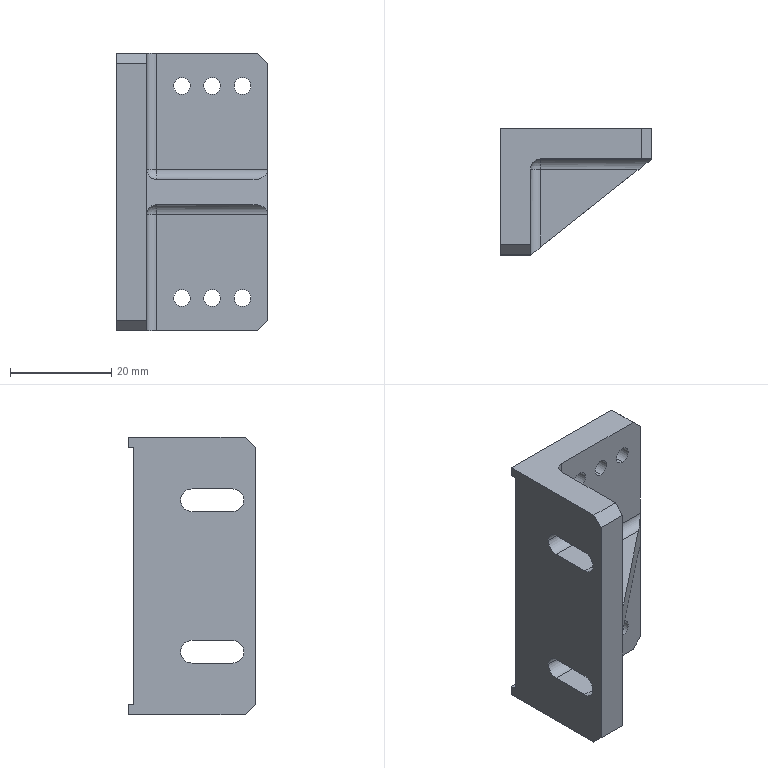Part | STEP file | 11-FG-SZ00811 | 1 solid | 51 faces | box 30 x 25 x 55 mm | volume 14965 mm3 | plane 25 | cylinder 24 | sphere 2 | commonest cylinder face diameters 3.3 x12 4 x6 4.5 x6
STEP:
#1=CARTESIAN_POINT('',(0.,-10.25,42.5));
#2=VERTEX_POINT('',#1);
#3=CARTESIAN_POINT('',(0.,-12.5,44.75));
#4=VERTEX_POINT('',#3);
#5=CARTESIAN_POINT('',(0.,-12.5,42.5));
#6=DIRECTION('',(1.,0.,0.));
#7=DIRECTION('',(0.,-1.,0.));
#8=AXIS2_PLACEMENT_3D('',#5,#6,#7);
#9=CIRCLE('',#8,2.25);
#10=EDGE_CURVE('',#2,#4,#9,.T.);
#11=ORIENTED_EDGE('',*,*,#10,.F.);
#12=CARTESIAN_POINT('',(6.,-10.25,42.5));
#13=VERTEX_POINT('',#12);
#14=CARTESIAN_POINT('',(0.,-10.25,42.5));
#15=DIRECTION('',(1.,0.,0.));
#16=VECTOR('',#15,1000.);
#17=LINE('',#14,#16);
#18=EDGE_CURVE('',#2,#13,#17,.T.);
#19=ORIENTED_EDGE('',*,*,#18,.T.);
#20=CARTESIAN_POINT('',(6.,-12.5,44.75));
#21=VERTEX_POINT('',#20);
#22=CARTESIAN_POINT('',(6.,-12.5,42.5));
#23=DIRECTION('',(1.,0.,0.));
#24=DIRECTION('',(0.,-1.,0.));
#25=AXIS2_PLACEMENT_3D('',#22,#23,#24);
#26=CIRCLE('',#25,2.25);
#27=EDGE_CURVE('',#13,#21,#26,.T.);
#28=ORIENTED_EDGE('',*,*,#27,.T.);
#29=CARTESIAN_POINT('',(0.,-12.5,44.75));
#30=DIRECTION('',(1.,0.,0.));
#31=VECTOR('',#30,1000.);
#32=LINE('',#29,#31);
#33=EDGE_CURVE('',#4,#21,#32,.T.);
#34=ORIENTED_EDGE('',*,*,#33,.F.);
#35=EDGE_LOOP('',(#11,#19,#28,#34));
#36=FACE_OUTER_BOUND('',#35,.T.);
#37=CARTESIAN_POINT('',(0.,-12.5,42.5));
#38=DIRECTION('',(1.,0.,0.));
#39=DIRECTION('',(0.,1.,0.));
#40=AXIS2_PLACEMENT_3D('',#37,#38,#39);
#41=CYLINDRICAL_SURFACE('',#40,2.25);
#42=ADVANCED_FACE('',(#36),#41,.F.);
#43=CARTESIAN_POINT('',(0.,-10.25,12.5));
#44=VERTEX_POINT('',#43);
#45=CARTESIAN_POINT('',(0.,-12.5,14.75));
#46=VERTEX_POINT('',#45);
#47=CARTESIAN_POINT('',(0.,-12.5,12.5));
#48=DIRECTION('',(1.,0.,0.));
#49=DIRECTION('',(0.,1.,0.));
#50=AXIS2_PLACEMENT_3D('',#47,#48,#49);
#51=CIRCLE('',#50,2.25);
#52=EDGE_CURVE('',#44,#46,#51,.T.);
#53=ORIENTED_EDGE('',*,*,#52,.F.);
#54=CARTESIAN_POINT('',(6.,-10.25,12.5));
#55=VERTEX_POINT('',#54);
#56=CARTESIAN_POINT('',(0.,-10.25,12.5));
#57=DIRECTION('',(1.,0.,0.));
#58=VECTOR('',#57,1000.);
#59=LINE('',#56,#58);
#60=EDGE_CURVE('',#44,#55,#59,.T.);
#61=ORIENTED_EDGE('',*,*,#60,.T.);
#62=CARTESIAN_POINT('',(6.,-12.5,14.75));
#63=VERTEX_POINT('',#62);
#64=CARTESIAN_POINT('',(6.,-12.5,12.5));
#65=DIRECTION('',(1.,0.,0.));
#66=DIRECTION('',(0.,1.,0.));
#67=AXIS2_PLACEMENT_3D('',#64,#65,#66);
#68=CIRCLE('',#67,2.25);
#69=EDGE_CURVE('',#55,#63,#68,.T.);
#70=ORIENTED_EDGE('',*,*,#69,.T.);
#71=CARTESIAN_POINT('',(0.,-12.5,14.75));
#72=DIRECTION('',(1.,0.,0.));
#73=VECTOR('',#72,1000.);
#74=LINE('',#71,#73);
#75=EDGE_CURVE('',#46,#63,#74,.T.);
#76=ORIENTED_EDGE('',*,*,#75,.F.);
#77=EDGE_LOOP('',(#53,#61,#70,#76));
#78=FACE_OUTER_BOUND('',#77,.T.);
#79=CARTESIAN_POINT('',(0.,-12.5,12.5));
#80=DIRECTION('',(1.,0.,0.));
#81=DIRECTION('',(0.,1.,0.));
#82=AXIS2_PLACEMENT_3D('',#79,#80,#81);
#83=CYLINDRICAL_SURFACE('',#82,2.25);
#84=ADVANCED_FACE('',(#78),#83,.F.);
#85=CARTESIAN_POINT('',(13.,-6.,4.85));
#86=VERTEX_POINT('',#85);
#87=CARTESIAN_POINT('',(13.,-6.,8.15));
#88=VERTEX_POINT('',#87);
#89=CARTESIAN_POINT('',(13.,-6.,6.5));
#90=DIRECTION('',(0.,1.,0.));
#91=DIRECTION('',(0.,0.,1.));
#92=AXIS2_PLACEMENT_3D('',#89,#90,#91);
#93=CIRCLE('',#92,1.65);
#94=EDGE_CURVE('',#86,#88,#93,.T.);
#95=ORIENTED_EDGE('',*,*,#94,.F.);
#96=CARTESIAN_POINT('',(13.,-1.,4.85));
#97=VERTEX_POINT('',#96);
#98=CARTESIAN_POINT('',(13.,-1.,4.85));
#99=DIRECTION('',(0.,1.,0.));
#100=VECTOR('',#99,1000.);
#101=LINE('',#98,#100);
#102=EDGE_CURVE('',#86,#97,#101,.T.);
#103=ORIENTED_EDGE('',*,*,#102,.T.);
#104=CARTESIAN_POINT('',(13.,-1.,8.15));
#105=VERTEX_POINT('',#104);
#106=CARTESIAN_POINT('',(13.,-1.,6.5));
#107=DIRECTION('',(0.,1.,0.));
#108=DIRECTION('',(0.,0.,1.));
#109=AXIS2_PLACEMENT_3D('',#106,#107,#108);
#110=CIRCLE('',#109,1.65);
#111=EDGE_CURVE('',#97,#105,#110,.T.);
#112=ORIENTED_EDGE('',*,*,#111,.T.);
#113=CARTESIAN_POINT('',(13.,-1.,8.15));
#114=DIRECTION('',(0.,1.,0.));
#115=VECTOR('',#114,1000.);
#116=LINE('',#113,#115);
#117=EDGE_CURVE('',#88,#105,#116,.T.);
#118=ORIENTED_EDGE('',*,*,#117,.F.);
#119=EDGE_LOOP('',(#95,#103,#112,#118));
#120=FACE_OUTER_BOUND('',#119,.T.);
#121=CARTESIAN_POINT('',(13.,-1.,6.5));
#122=DIRECTION('',(0.,1.,0.));
#123=DIRECTION('',(0.,0.,1.));
#124=AXIS2_PLACEMENT_3D('',#121,#122,#123);
#125=CYLINDRICAL_SURFACE('',#124,1.65);
#126=ADVANCED_FACE('',(#120),#125,.F.);
#127=CARTESIAN_POINT('',(13.,-6.,46.85));
#128=VERTEX_POINT('',#127);
#129=CARTESIAN_POINT('',(13.,-6.,50.15));
#130=VERTEX_POINT('',#129);
#131=CARTESIAN_POINT('',(13.,-6.,48.5));
#132=DIRECTION('',(0.,1.,0.));
#133=DIRECTION('',(0.,0.,1.));
#134=AXIS2_PLACEMENT_3D('',#131,#132,#133);
#135=CIRCLE('',#134,1.65);
#136=EDGE_CURVE('',#128,#130,#135,.T.);
#137=ORIENTED_EDGE('',*,*,#136,.F.);
#138=CARTESIAN_POINT('',(13.,-1.,46.85));
#139=VERTEX_POINT('',#138);
#140=CARTESIAN_POINT('',(13.,-1.,46.85));
#141=DIRECTION('',(0.,1.,0.));
#142=VECTOR('',#141,1000.);
#143=LINE('',#140,#142);
#144=EDGE_CURVE('',#128,#139,#143,.T.);
#145=ORIENTED_EDGE('',*,*,#144,.T.);
#146=CARTESIAN_POINT('',(13.,-1.,50.15));
#147=VERTEX_POINT('',#146);
#148=CARTESIAN_POINT('',(13.,-1.,48.5));
#149=DIRECTION('',(0.,1.,0.));
#150=DIRECTION('',(0.,0.,1.));
#151=AXIS2_PLACEMENT_3D('',#148,#149,#150);
#152=CIRCLE('',#151,1.65);
#153=EDGE_CURVE('',#139,#147,#152,.T.);
#154=ORIENTED_EDGE('',*,*,#153,.T.);
#155=CARTESIAN_POINT('',(13.,-1.,50.15));
#156=DIRECTION('',(0.,1.,0.));
#157=VECTOR('',#156,1000.);
#158=LINE('',#155,#157);
#159=EDGE_CURVE('',#130,#147,#158,.T.);
#160=ORIENTED_EDGE('',*,*,#159,.F.);
#161=EDGE_LOOP('',(#137,#145,#154,#160));
#162=FACE_OUTER_BOUND('',#161,.T.);
#163=CARTESIAN_POINT('',(13.,-1.,48.5));
#164=DIRECTION('',(0.,1.,0.));
#165=DIRECTION('',(0.,0.,1.));
#166=AXIS2_PLACEMENT_3D('',#163,#164,#165);
#167=CYLINDRICAL_SURFACE('',#166,1.65);
#168=ADVANCED_FACE('',(#162),#167,.F.);
#169=CARTESIAN_POINT('',(19.,-6.,4.85));
#170=VERTEX_POINT('',#169);
#171=CARTESIAN_POINT('',(19.,-6.,8.15));
#172=VERTEX_POINT('',#171);
#173=CARTESIAN_POINT('',(19.,-6.,6.5));
#174=DIRECTION('',(0.,1.,0.));
#175=DIRECTION('',(0.,0.,1.));
#176=AXIS2_PLACEMENT_3D('',#173,#174,#175);
#177=CIRCLE('',#176,1.65);
#178=EDGE_CURVE('',#170,#172,#177,.T.);
#179=ORIENTED_EDGE('',*,*,#178,.F.);
#180=CARTESIAN_POINT('',(19.,-1.,4.85));
#181=VERTEX_POINT('',#180);
#182=CARTESIAN_POINT('',(19.,-1.,4.85));
#183=DIRECTION('',(0.,1.,0.));
#184=VECTOR('',#183,1000.);
#185=LINE('',#182,#184);
#186=EDGE_CURVE('',#170,#181,#185,.T.);
#187=ORIENTED_EDGE('',*,*,#186,.T.);
#188=CARTESIAN_POINT('',(19.,-1.,8.15));
#189=VERTEX_POINT('',#188);
#190=CARTESIAN_POINT('',(19.,-1.,6.5));
#191=DIRECTION('',(0.,1.,0.));
#192=DIRECTION('',(0.,0.,1.));
#193=AXIS2_PLACEMENT_3D('',#190,#191,#192);
#194=CIRCLE('',#193,1.65);
#195=EDGE_CURVE('',#181,#189,#194,.T.);
#196=ORIENTED_EDGE('',*,*,#195,.T.);
#197=CARTESIAN_POINT('',(19.,-1.,8.15));
#198=DIRECTION('',(0.,1.,0.));
#199=VECTOR('',#198,1000.);
#200=LINE('',#197,#199);
#201=EDGE_CURVE('',#172,#189,#200,.T.);
#202=ORIENTED_EDGE('',*,*,#201,.F.);
#203=EDGE_LOOP('',(#179,#187,#196,#202));
#204=FACE_OUTER_BOUND('',#203,.T.);
#205=CARTESIAN_POINT('',(19.,-1.,6.5));
#206=DIRECTION('',(0.,1.,0.));
#207=DIRECTION('',(0.,0.,1.));
#208=AXIS2_PLACEMENT_3D('',#205,#206,#207);
#209=CYLINDRICAL_SURFACE('',#208,1.65);
#210=ADVANCED_FACE('',(#204),#209,.F.);
#211=CARTESIAN_POINT('',(19.,-6.,46.85));
#212=VERTEX_POINT('',#211);
#213=CARTESIAN_POINT('',(19.,-6.,50.15));
#214=VERTEX_POINT('',#213);
#215=CARTESIAN_POINT('',(19.,-6.,48.5));
#216=DIRECTION('',(0.,1.,0.));
#217=DIRECTION('',(0.,0.,1.));
#218=AXIS2_PLACEMENT_3D('',#215,#216,#217);
#219=CIRCLE('',#218,1.65);
#220=EDGE_CURVE('',#212,#214,#219,.T.);
#221=ORIENTED_EDGE('',*,*,#220,.F.);
#222=CARTESIAN_POINT('',(19.,-1.,46.85));
#223=VERTEX_POINT('',#222);
#224=CARTESIAN_POINT('',(19.,-1.,46.85));
#225=DIRECTION('',(0.,1.,0.));
#226=VECTOR('',#225,1000.);
#227=LINE('',#224,#226);
#228=EDGE_CURVE('',#212,#223,#227,.T.);
#229=ORIENTED_EDGE('',*,*,#228,.T.);
#230=CARTESIAN_POINT('',(19.,-1.,50.15));
#231=VERTEX_POINT('',#230);
#232=CARTESIAN_POINT('',(19.,-1.,48.5));
#233=DIRECTION('',(0.,1.,0.));
#234=DIRECTION('',(0.,0.,1.));
#235=AXIS2_PLACEMENT_3D('',#232,#233,#234);
#236=CIRCLE('',#235,1.65);
#237=EDGE_CURVE('',#223,#231,#236,.T.);
#238=ORIENTED_EDGE('',*,*,#237,.T.);
#239=CARTESIAN_POINT('',(19.,-1.,50.15));
#240=DIRECTION('',(0.,1.,0.));
#241=VECTOR('',#240,1000.);
#242=LINE('',#239,#241);
#243=EDGE_CURVE('',#214,#231,#242,.T.);
#244=ORIENTED_EDGE('',*,*,#243,.F.);
#245=EDGE_LOOP('',(#221,#229,#238,#244));
#246=FACE_OUTER_BOUND('',#245,.T.);
#247=CARTESIAN_POINT('',(19.,-1.,48.5));
#248=DIRECTION('',(0.,1.,0.));
#249=DIRECTION('',(0.,0.,1.));
#250=AXIS2_PLACEMENT_3D('',#247,#248,#249);
#251=CYLINDRICAL_SURFACE('',#250,1.65);
#252=ADVANCED_FACE('',(#246),#251,.F.);
#253=CARTESIAN_POINT('',(25.,-6.,4.85));
#254=VERTEX_POINT('',#253);
#255=CARTESIAN_POINT('',(25.,-6.,8.15));
#256=VERTEX_POINT('',#255);
#257=CARTESIAN_POINT('',(25.,-6.,6.5));
#258=DIRECTION('',(0.,1.,0.));
#259=DIRECTION('',(0.,0.,1.));
#260=AXIS2_PLACEMENT_3D('',#257,#258,#259);
#261=CIRCLE('',#260,1.65);
#262=EDGE_CURVE('',#254,#256,#261,.T.);
#263=ORIENTED_EDGE('',*,*,#262,.F.);
#264=CARTESIAN_POINT('',(25.,-1.,4.85));
#265=VERTEX_POINT('',#264);
#266=CARTESIAN_POINT('',(25.,-1.,4.85));
#267=DIRECTION('',(0.,1.,0.));
#268=VECTOR('',#267,1000.);
#269=LINE('',#266,#268);
#270=EDGE_CURVE('',#254,#265,#269,.T.);
#271=ORIENTED_EDGE('',*,*,#270,.T.);
#272=CARTESIAN_POINT('',(25.,-1.,8.15));
#273=VERTEX_POINT('',#272);
#274=CARTESIAN_POINT('',(25.,-1.,6.5));
#275=DIRECTION('',(0.,1.,0.));
#276=DIRECTION('',(0.,0.,1.));
#277=AXIS2_PLACEMENT_3D('',#274,#275,#276);
#278=CIRCLE('',#277,1.65);
#279=EDGE_CURVE('',#265,#273,#278,.T.);
#280=ORIENTED_EDGE('',*,*,#279,.T.);
#281=CARTESIAN_POINT('',(25.,-1.,8.15));
#282=DIRECTION('',(0.,1.,0.));
#283=VECTOR('',#282,1000.);
#284=LINE('',#281,#283);
#285=EDGE_CURVE('',#256,#273,#284,.T.);
#286=ORIENTED_EDGE('',*,*,#285,.F.);
#287=EDGE_LOOP('',(#263,#271,#280,#286));
#288=FACE_OUTER_BOUND('',#287,.T.);
#289=CARTESIAN_POINT('',(25.,-1.,6.5));
#290=DIRECTION('',(0.,1.,0.));
#291=DIRECTION('',(0.,0.,1.));
#292=AXIS2_PLACEMENT_3D('',#289,#290,#291);
#293=CYLINDRICAL_SURFACE('',#292,1.65);
#294=ADVANCED_FACE('',(#288),#293,.F.);
#295=CARTESIAN_POINT('',(25.,-6.,46.85));
#296=VERTEX_POINT('',#295);
#297=CARTESIAN_POINT('',(25.,-6.,50.15));
#298=VERTEX_POINT('',#297);
#299=CARTESIAN_POINT('',(25.,-6.,48.5));
#300=DIRECTION('',(0.,1.,0.));
#301=DIRECTION('',(0.,0.,1.));
#302=AXIS2_PLACEMENT_3D('',#299,#300,#301);
#303=CIRCLE('',#302,1.65);
#304=EDGE_CURVE('',#296,#298,#303,.T.);
#305=ORIENTED_EDGE('',*,*,#304,.F.);
#306=CARTESIAN_POINT('',(25.,-1.,46.85));
#307=VERTEX_POINT('',#306);
#308=CARTESIAN_POINT('',(25.,-1.,46.85));
#309=DIRECTION('',(0.,1.,0.));
#310=VECTOR('',#309,1000.);
#311=LINE('',#308,#310);
#312=EDGE_CURVE('',#296,#307,#311,.T.);
#313=ORIENTED_EDGE('',*,*,#312,.T.);
#314=CARTESIAN_POINT('',(25.,-1.,50.15));
#315=VERTEX_POINT('',#314);
#316=CARTESIAN_POINT('',(25.,-1.,48.5));
#317=DIRECTION('',(0.,1.,0.));
#318=DIRECTION('',(0.,0.,1.));
#319=AXIS2_PLACEMENT_3D('',#316,#317,#318);
#320=CIRCLE('',#319,1.65);
#321=EDGE_CURVE('',#307,#315,#320,.T.);
#322=ORIENTED_EDGE('',*,*,#321,.T.);
#323=CARTESIAN_POINT('',(25.,-1.,50.15));
#324=DIRECTION('',(0.,1.,0.));
#325=VECTOR('',#324,1000.);
#326=LINE('',#323,#325);
#327=EDGE_CURVE('',#298,#315,#326,.T.);
#328=ORIENTED_EDGE('',*,*,#327,.F.);
#329=EDGE_LOOP('',(#305,#313,#322,#328));
#330=FACE_OUTER_BOUND('',#329,.T.);
#331=CARTESIAN_POINT('',(25.,-1.,48.5));
#332=DIRECTION('',(0.,1.,0.));
#333=DIRECTION('',(0.,0.,1.));
#334=AXIS2_PLACEMENT_3D('',#331,#332,#333);
#335=CYLINDRICAL_SURFACE('',#334,1.65);
#336=ADVANCED_FACE('',(#330),#335,.F.);
#337=CARTESIAN_POINT('',(13.,-6.,48.5));
#338=DIRECTION('',(0.,1.,0.));
#339=DIRECTION('',(0.,0.,1.));
#340=AXIS2_PLACEMENT_3D('',#337,#338,#339);
#341=CIRCLE('',#340,1.65);
#342=EDGE_CURVE('',#130,#128,#341,.T.);
#343=ORIENTED_EDGE('',*,*,#342,.T.);
#344=ORIENTED_EDGE('',*,*,#136,.T.);
#345=EDGE_LOOP('',(#343,#344));
#346=FACE_BOUND('',#345,.T.);
#347=CARTESIAN_POINT('',(19.,-6.,48.5));
#348=DIRECTION('',(0.,1.,0.));
#349=DIRECTION('',(0.,0.,1.));
#350=AXIS2_PLACEMENT_3D('',#347,#348,#349);
#351=CIRCLE('',#350,1.65);
#352=EDGE_CURVE('',#214,#212,#351,.T.);
#353=ORIENTED_EDGE('',*,*,#352,.T.);
#354=ORIENTED_EDGE('',*,*,#220,.T.);
#355=EDGE_LOOP('',(#353,#354));
#356=FACE_BOUND('',#355,.T.);
#357=CARTESIAN_POINT('',(25.,-6.,48.5));
#358=DIRECTION('',(0.,1.,0.));
#359=DIRECTION('',(0.,0.,1.));
#360=AXIS2_PLACEMENT_3D('',#357,#358,#359);
#361=CIRCLE('',#360,1.65);
#362=EDGE_CURVE('',#298,#296,#361,.T.);
#363=ORIENTED_EDGE('',*,*,#362,.T.);
#364=ORIENTED_EDGE('',*,*,#304,.T.);
#365=EDGE_LOOP('',(#363,#364));
#366=FACE_BOUND('',#365,.T.);
#367=CARTESIAN_POINT('',(30.,-6.,53.));
#368=VERTEX_POINT('',#367);
#369=CARTESIAN_POINT('',(30.,-6.,32.));
#370=VERTEX_POINT('',#369);
#371=CARTESIAN_POINT('',(30.,-6.,55.));
#372=DIRECTION('',(0.,0.,-1.));
#373=VECTOR('',#372,1000.);
#374=LINE('',#371,#373);
#375=EDGE_CURVE('',#368,#370,#374,.T.);
#376=ORIENTED_EDGE('',*,*,#375,.F.);
#377=CARTESIAN_POINT('',(28.,-6.,55.));
#378=VERTEX_POINT('',#377);
#379=CARTESIAN_POINT('',(30.,-6.,53.));
#380=DIRECTION('',(-0.7071,0.,0.7071));
#381=VECTOR('',#380,1000.);
#382=LINE('',#379,#381);
#383=EDGE_CURVE('',#368,#378,#382,.T.);
#384=ORIENTED_EDGE('',*,*,#383,.T.);
#385=CARTESIAN_POINT('',(8.,-6.,55.));
#386=VERTEX_POINT('',#385);
#387=CARTESIAN_POINT('',(0.,-6.,55.));
#388=DIRECTION('',(1.,0.,0.));
#389=VECTOR('',#388,1000.);
#390=LINE('',#387,#389);
#391=EDGE_CURVE('',#386,#378,#390,.T.);
#392=ORIENTED_EDGE('',*,*,#391,.F.);
#393=CARTESIAN_POINT('',(8.,-6.,32.));
#394=VERTEX_POINT('',#393);
#395=CARTESIAN_POINT('',(8.,-6.,30.));
#396=DIRECTION('',(0.,0.,-1.));
#397=VECTOR('',#396,1000.);
#398=LINE('',#395,#397);
#399=EDGE_CURVE('',#386,#394,#398,.T.);
#400=ORIENTED_EDGE('',*,*,#399,.T.);
#401=CARTESIAN_POINT('',(30.,-6.,32.));
#402=DIRECTION('',(1.,0.,0.));
#403=VECTOR('',#402,1000.);
#404=LINE('',#401,#403);
#405=EDGE_CURVE('',#394,#370,#404,.T.);
#406=ORIENTED_EDGE('',*,*,#405,.T.);
#407=EDGE_LOOP('',(#376,#384,#392,#400,#406));
#408=FACE_OUTER_BOUND('',#407,.T.);
#409=CARTESIAN_POINT('',(0.,-6.,55.));
#410=DIRECTION('',(0.,1.,0.));
#411=DIRECTION('',(0.,0.,1.));
#412=AXIS2_PLACEMENT_3D('',#409,#410,#411);
#413=PLANE('',#412);
#414=ADVANCED_FACE('',(#346,#356,#366,#408),#413,.F.);
#415=CARTESIAN_POINT('',(6.,-20.5,40.25));
#416=VERTEX_POINT('',#415);
#417=CARTESIAN_POINT('',(6.,-12.5,40.25));
#418=VERTEX_POINT('',#417);
#419=CARTESIAN_POINT('',(6.,-20.5,40.25));
#420=DIRECTION('',(0.,1.,0.));
#421=VECTOR('',#420,1000.);
#422=LINE('',#419,#421);
#423=EDGE_CURVE('',#416,#418,#422,.T.);
#424=ORIENTED_EDGE('',*,*,#423,.F.);
#425=CARTESIAN_POINT('',(6.,-20.5,44.75));
#426=VERTEX_POINT('',#425);
#427=CARTESIAN_POINT('',(6.,-20.5,42.5));
#428=DIRECTION('',(1.,0.,0.));
#429=DIRECTION('',(0.,-1.,0.));
#430=AXIS2_PLACEMENT_3D('',#427,#428,#429);
#431=CIRCLE('',#430,2.25);
#432=EDGE_CURVE('',#426,#416,#431,.T.);
#433=ORIENTED_EDGE('',*,*,#432,.F.);
#434=CARTESIAN_POINT('',(6.,-20.5,44.75));
#435=DIRECTION('',(0.,-1.,0.));
#436=VECTOR('',#435,1000.);
#437=LINE('',#434,#436);
#438=EDGE_CURVE('',#21,#426,#437,.T.);
#439=ORIENTED_EDGE('',*,*,#438,.F.);
#440=ORIENTED_EDGE('',*,*,#27,.F.);
#441=CARTESIAN_POINT('',(6.,-12.5,42.5));
#442=DIRECTION('',(1.,0.,0.));
#443=DIRECTION('',(0.,-1.,0.));
#444=AXIS2_PLACEMENT_3D('',#441,#442,#443);
#445=CIRCLE('',#444,2.25);
#446=EDGE_CURVE('',#418,#13,#445,.T.);
#447=ORIENTED_EDGE('',*,*,#446,.F.);
#448=EDGE_LOOP('',(#424,#433,#439,#440,#447));
#449=FACE_BOUND('',#448,.T.);
#450=CARTESIAN_POINT('',(6.,-23.,55.));
#451=VERTEX_POINT('',#450);
#452=CARTESIAN_POINT('',(6.,-8.,55.));
#453=VERTEX_POINT('',#452);
#454=CARTESIAN_POINT('',(6.,0.,55.));
#455=DIRECTION('',(0.,1.,0.));
#456=VECTOR('',#455,1000.);
#457=LINE('',#454,#456);
#458=EDGE_CURVE('',#451,#453,#457,.T.);
#459=ORIENTED_EDGE('',*,*,#458,.F.);
#460=CARTESIAN_POINT('',(6.,-25.,53.));
#461=VERTEX_POINT('',#460);
#462=CARTESIAN_POINT('',(6.,-25.,53.));
#463=DIRECTION('',(0.,-0.7071,-0.7071));
#464=VECTOR('',#463,1000.);
#465=LINE('',#462,#464);
#466=EDGE_CURVE('',#451,#461,#465,.T.);
#467=ORIENTED_EDGE('',*,*,#466,.T.);
#468=CARTESIAN_POINT('',(6.,-25.,32.));
#469=VERTEX_POINT('',#468);
#470=CARTESIAN_POINT('',(6.,-25.,55.));
#471=DIRECTION('',(0.,0.,-1.));
#472=VECTOR('',#471,1000.);
#473=LINE('',#470,#472);
#474=EDGE_CURVE('',#461,#469,#473,.T.);
#475=ORIENTED_EDGE('',*,*,#474,.T.);
#476=CARTESIAN_POINT('',(6.,-8.,32.));
#477=VERTEX_POINT('',#476);
#478=CARTESIAN_POINT('',(6.,-6.,32.));
#479=DIRECTION('',(0.,1.,0.));
#480=VECTOR('',#479,1000.);
#481=LINE('',#478,#480);
#482=EDGE_CURVE('',#469,#477,#481,.T.);
#483=ORIENTED_EDGE('',*,*,#482,.T.);
#484=CARTESIAN_POINT('',(6.,-8.,55.));
#485=DIRECTION('',(0.,0.,1.));
#486=VECTOR('',#485,1000.);
#487=LINE('',#484,#486);
#488=EDGE_CURVE('',#477,#453,#487,.T.);
#489=ORIENTED_EDGE('',*,*,#488,.T.);
#490=EDGE_LOOP('',(#459,#467,#475,#483,#489));
#491=FACE_OUTER_BOUND('',#490,.T.);
#492=CARTESIAN_POINT('',(6.,0.,55.));
#493=DIRECTION('',(-1.,0.,0.));
#494=DIRECTION('',(0.,-1.,0.));
#495=AXIS2_PLACEMENT_3D('',#492,#493,#494);
#496=PLANE('',#495);
#497=ADVANCED_FACE('',(#449,#491),#496,.F.);
#498=CARTESIAN_POINT('',(13.,-1.,6.5));
#499=DIRECTION('',(0.,1.,0.));
#500=DIRECTION('',(0.,0.,1.));
#501=AXIS2_PLACEMENT_3D('',#498,#499,#500);
#502=CIRCLE('',#501,1.65);
#503=EDGE_CURVE('',#105,#97,#502,.T.);
#504=ORIENTED_EDGE('',*,*,#503,.F.);
#505=ORIENTED_EDGE('',*,*,#111,.F.);
#506=EDGE_LOOP('',(#504,#505));
#507=FACE_BOUND('',#506,.T.);
#508=CARTESIAN_POINT('',(13.,-1.,48.5));
#509=DIRECTION('',(0.,1.,0.));
#510=DIRECTION('',(0.,0.,1.));
#511=AXIS2_PLACEMENT_3D('',#508,#509,#510);
#512=CIRCLE('',#511,1.65);
#513=EDGE_CURVE('',#147,#139,#512,.T.);
#514=ORIENTED_EDGE('',*,*,#513,.F.);
#515=ORIENTED_EDGE('',*,*,#153,.F.);
#516=EDGE_LOOP('',(#514,#515));
#517=FACE_BOUND('',#516,.T.);
#518=CARTESIAN_POINT('',(19.,-1.,48.5));
#519=DIRECTION('',(0.,1.,0.));
#520=DIRECTION('',(0.,0.,1.));
#521=AXIS2_PLACEMENT_3D('',#518,#519,#520);
#522=CIRCLE('',#521,1.65);
#523=EDGE_CURVE('',#231,#223,#522,.T.);
#524=ORIENTED_EDGE('',*,*,#523,.F.);
#525=ORIENTED_EDGE('',*,*,#237,.F.);
#526=EDGE_LOOP('',(#524,#525));
#527=FACE_BOUND('',#526,.T.);
#528=CARTESIAN_POINT('',(25.,-1.,6.5));
#529=DIRECTION('',(0.,1.,0.));
#530=DIRECTION('',(0.,0.,1.));
#531=AXIS2_PLACEMENT_3D('',#528,#529,#530);
#532=CIRCLE('',#531,1.65);
#533=EDGE_CURVE('',#273,#265,#532,.T.);
#534=ORIENTED_EDGE('',*,*,#533,.F.);
#535=ORIENTED_EDGE('',*,*,#279,.F.);
#536=EDGE_LOOP('',(#534,#535));
#537=FACE_BOUND('',#536,.T.);
#538=CARTESIAN_POINT('',(25.,-1.,48.5));
#539=DIRECTION('',(0.,1.,0.));
#540=DIRECTION('',(0.,0.,1.));
#541=AXIS2_PLACEMENT_3D('',#538,#539,#540);
#542=CIRCLE('',#541,1.65);
#543=EDGE_CURVE('',#315,#307,#542,.T.);
#544=ORIENTED_EDGE('',*,*,#543,.F.);
#545=ORIENTED_EDGE('',*,*,#321,.F.);
#546=EDGE_LOOP('',(#544,#545));
#547=FACE_BOUND('',#546,.T.);
#548=CARTESIAN_POINT('',(0.,-1.,2.));
#549=VERTEX_POINT('',#548);
#550=CARTESIAN_POINT('',(0.,-1.,53.));
#551=VERTEX_POINT('',#550);
#552=CARTESIAN_POINT('',(0.,-1.,2.));
#553=DIRECTION('',(0.,0.,1.));
#554=VECTOR('',#553,1000.);
#555=LINE('',#552,#554);
#556=EDGE_CURVE('',#549,#551,#555,.T.);
#557=ORIENTED_EDGE('',*,*,#556,.T.);
#558=CARTESIAN_POINT('',(30.,-1.,53.));
#559=VERTEX_POINT('',#558);
#560=CARTESIAN_POINT('',(30.,-1.,53.));
#561=DIRECTION('',(-1.,0.,0.));
#562=VECTOR('',#561,1000.);
#563=LINE('',#560,#562);
#564=EDGE_CURVE('',#559,#551,#563,.T.);
#565=ORIENTED_EDGE('',*,*,#564,.F.);
#566=CARTESIAN_POINT('',(30.,-1.,2.));
#567=VERTEX_POINT('',#566);
#568=CARTESIAN_POINT('',(30.,-1.,2.));
#569=DIRECTION('',(0.,0.,1.));
#570=VECTOR('',#569,1000.);
#571=LINE('',#568,#570);
#572=EDGE_CURVE('',#567,#559,#571,.T.);
#573=ORIENTED_EDGE('',*,*,#572,.F.);
#574=CARTESIAN_POINT('',(30.,-1.,2.));
#575=DIRECTION('',(-1.,0.,0.));
#576=VECTOR('',#575,1000.);
#577=LINE('',#574,#576);
#578=EDGE_CURVE('',#567,#549,#577,.T.);
#579=ORIENTED_EDGE('',*,*,#578,.T.);
#580=EDGE_LOOP('',(#557,#565,#573,#579));
#581=FACE_OUTER_BOUND('',#580,.T.);
#582=CARTESIAN_POINT('',(19.,-1.,6.5));
#583=DIRECTION('',(0.,1.,0.));
#584=DIRECTION('',(0.,0.,1.));
#585=AXIS2_PLACEMENT_3D('',#582,#583,#584);
#586=CIRCLE('',#585,1.65);
#587=EDGE_CURVE('',#189,#181,#586,.T.);
#588=ORIENTED_EDGE('',*,*,#587,.F.);
#589=ORIENTED_EDGE('',*,*,#195,.F.);
#590=EDGE_LOOP('',(#588,#589));
#591=FACE_BOUND('',#590,.T.);
#592=CARTESIAN_POINT('',(30.,-1.,2.));
#593=DIRECTION('',(0.,-1.,0.));
#594=DIRECTION('',(0.,0.,-1.));
#595=AXIS2_PLACEMENT_3D('',#592,#593,#594);
#596=PLANE('',#595);
#597=ADVANCED_FACE('',(#507,#517,#527,#537,#547,#581,#591),#596,.F.);
#598=CARTESIAN_POINT('',(30.,0.,2.));
#599=VERTEX_POINT('',#598);
#600=CARTESIAN_POINT('',(0.,0.,2.));
#601=VERTEX_POINT('',#600);
#602=CARTESIAN_POINT('',(30.,0.,2.));
#603=DIRECTION('',(-1.,0.,0.));
#604=VECTOR('',#603,1000.);
#605=LINE('',#602,#604);
#606=EDGE_CURVE('',#599,#601,#605,.T.);
#607=ORIENTED_EDGE('',*,*,#606,.F.);
#608=CARTESIAN_POINT('',(28.,0.,0.));
#609=VERTEX_POINT('',#608);
#610=CARTESIAN_POINT('',(41.5,0.,13.5));
#611=DIRECTION('',(-0.7071,0.,-0.7071));
#612=VECTOR('',#611,1000.);
#613=LINE('',#610,#612);
#614=EDGE_CURVE('',#599,#609,#613,.T.);
#615=ORIENTED_EDGE('',*,*,#614,.T.);
#616=CARTESIAN_POINT('',(0.,0.,0.));
#617=VERTEX_POINT('',#616);
#618=CARTESIAN_POINT('',(0.,0.,0.));
#619=DIRECTION('',(1.,0.,0.));
#620=VECTOR('',#619,1000.);
#621=LINE('',#618,#620);
#622=EDGE_CURVE('',#617,#609,#621,.T.);
#623=ORIENTED_EDGE('',*,*,#622,.F.);
#624=CARTESIAN_POINT('',(0.,0.,55.));
#625=DIRECTION('',(0.,0.,-1.));
#626=VECTOR('',#625,1000.);
#627=LINE('',#624,#626);
#628=EDGE_CURVE('',#601,#617,#627,.T.);
#629=ORIENTED_EDGE('',*,*,#628,.F.);
#630=EDGE_LOOP('',(#607,#615,#623,#629));
#631=FACE_OUTER_BOUND('',#630,.T.);
#632=CARTESIAN_POINT('',(0.,0.,55.));
#633=DIRECTION('',(0.,1.,0.));
#634=DIRECTION('',(0.,0.,1.));
#635=AXIS2_PLACEMENT_3D('',#632,#633,#634);
#636=PLANE('',#635);
#637=ADVANCED_FACE('',(#631),#636,.T.);
#638=CARTESIAN_POINT('',(13.,-6.,6.5));
#639=DIRECTION('',(0.,1.,0.));
#640=DIRECTION('',(0.,0.,1.));
#641=AXIS2_PLACEMENT_3D('',#638,#639,#640);
#642=CIRCLE('',#641,1.65);
#643=EDGE_CURVE('',#88,#86,#642,.T.);
#644=ORIENTED_EDGE('',*,*,#643,.T.);
#645=ORIENTED_EDGE('',*,*,#94,.T.);
#646=EDGE_LOOP('',(#644,#645));
#647=FACE_BOUND('',#646,.T.);
#648=CARTESIAN_POINT('',(19.,-6.,6.5));
#649=DIRECTION('',(0.,1.,0.));
#650=DIRECTION('',(0.,0.,1.));
#651=AXIS2_PLACEMENT_3D('',#648,#649,#650);
#652=CIRCLE('',#651,1.65);
#653=EDGE_CURVE('',#172,#170,#652,.T.);
#654=ORIENTED_EDGE('',*,*,#653,.T.);
#655=ORIENTED_EDGE('',*,*,#178,.T.);
#656=EDGE_LOOP('',(#654,#655));
#657=FACE_BOUND('',#656,.T.);
#658=CARTESIAN_POINT('',(25.,-6.,6.5));
#659=DIRECTION('',(0.,1.,0.));
#660=DIRECTION('',(0.,0.,1.));
#661=AXIS2_PLACEMENT_3D('',#658,#659,#660);
#662=CIRCLE('',#661,1.65);
#663=EDGE_CURVE('',#256,#254,#662,.T.);
#664=ORIENTED_EDGE('',*,*,#663,.T.);
#665=ORIENTED_EDGE('',*,*,#262,.T.);
#666=EDGE_LOOP('',(#664,#665));
#667=FACE_BOUND('',#666,.T.);
#668=CARTESIAN_POINT('',(8.,-6.,0.));
#669=VERTEX_POINT('',#668);
#670=CARTESIAN_POINT('',(28.,-6.,0.));
#671=VERTEX_POINT('',#670);
#672=CARTESIAN_POINT('',(0.,-6.,0.));
#673=DIRECTION('',(1.,0.,0.));
#674=VECTOR('',#673,1000.);
#675=LINE('',#672,#674);
#676=EDGE_CURVE('',#669,#671,#675,.T.);
#677=ORIENTED_EDGE('',*,*,#676,.T.);
#678=CARTESIAN_POINT('',(30.,-6.,2.));
#679=VERTEX_POINT('',#678);
#680=CARTESIAN_POINT('',(28.,-6.,0.));
#681=DIRECTION('',(0.7071,0.,0.7071));
#682=VECTOR('',#681,1000.);
#683=LINE('',#680,#682);
#684=EDGE_CURVE('',#671,#679,#683,.T.);
#685=ORIENTED_EDGE('',*,*,#684,.T.);
#686=CARTESIAN_POINT('',(30.,-6.,23.));
#687=VERTEX_POINT('',#686);
#688=CARTESIAN_POINT('',(30.,-6.,55.));
#689=DIRECTION('',(0.,0.,-1.));
#690=VECTOR('',#689,1000.);
#691=LINE('',#688,#690);
#692=EDGE_CURVE('',#687,#679,#691,.T.);
#693=ORIENTED_EDGE('',*,*,#692,.F.);
#694=CARTESIAN_POINT('',(8.,-6.,23.));
#695=VERTEX_POINT('',#694);
#696=CARTESIAN_POINT('',(0.,-6.,23.));
#697=DIRECTION('',(-1.,0.,0.));
#698=VECTOR('',#697,1000.);
#699=LINE('',#696,#698);
#700=EDGE_CURVE('',#687,#695,#699,.T.);
#701=ORIENTED_EDGE('',*,*,#700,.T.);
#702=CARTESIAN_POINT('',(8.,-6.,0.));
#703=DIRECTION('',(0.,0.,-1.));
#704=VECTOR('',#703,1000.);
#705=LINE('',#702,#704);
#706=EDGE_CURVE('',#695,#669,#705,.T.);
#707=ORIENTED_EDGE('',*,*,#706,.T.);
#708=EDGE_LOOP('',(#677,#685,#693,#701,#707));
#709=FACE_OUTER_BOUND('',#708,.T.);
#710=CARTESIAN_POINT('',(0.,-6.,55.));
#711=DIRECTION('',(0.,1.,0.));
#712=DIRECTION('',(0.,0.,1.));
#713=AXIS2_PLACEMENT_3D('',#710,#711,#712);
#714=PLANE('',#713);
#715=ADVANCED_FACE('',(#647,#657,#667,#709),#714,.F.);
#716=ORIENTED_EDGE('',*,*,#692,.T.);
#717=CARTESIAN_POINT('',(30.,0.,2.));
#718=DIRECTION('',(0.,1.,0.));
#719=VECTOR('',#718,1000.);
#720=LINE('',#717,#719);
#721=EDGE_CURVE('',#679,#567,#720,.T.);
#722=ORIENTED_EDGE('',*,*,#721,.T.);
#723=ORIENTED_EDGE('',*,*,#572,.T.);
#724=CARTESIAN_POINT('',(30.,-6.,53.));
#725=DIRECTION('',(0.,-1.,0.));
#726=VECTOR('',#725,1000.);
#727=LINE('',#724,#726);
#728=EDGE_CURVE('',#559,#368,#727,.T.);
#729=ORIENTED_EDGE('',*,*,#728,.T.);
#730=ORIENTED_EDGE('',*,*,#375,.T.);
#731=CARTESIAN_POINT('',(30.,-6.,30.));
#732=DIRECTION('',(0.,0.,-1.));
#733=VECTOR('',#732,1000.);
#734=LINE('',#731,#733);
#735=EDGE_CURVE('',#370,#687,#734,.T.);
#736=ORIENTED_EDGE('',*,*,#735,.T.);
#737=EDGE_LOOP('',(#716,#722,#723,#729,#730,#736));
#738=FACE_OUTER_BOUND('',#737,.T.);
#739=CARTESIAN_POINT('',(30.,0.,55.));
#740=DIRECTION('',(1.,0.,0.));
#741=DIRECTION('',(0.,0.,-1.));
#742=AXIS2_PLACEMENT_3D('',#739,#740,#741);
#743=PLANE('',#742);
#744=ADVANCED_FACE('',(#738),#743,.T.);
#745=CARTESIAN_POINT('',(0.,0.,55.));
#746=VERTEX_POINT('',#745);
#747=CARTESIAN_POINT('',(28.,0.,55.));
#748=VERTEX_POINT('',#747);
#749=CARTESIAN_POINT('',(0.,0.,55.));
#750=DIRECTION('',(1.,0.,0.));
#751=VECTOR('',#750,1000.);
#752=LINE('',#749,#751);
#753=EDGE_CURVE('',#746,#748,#752,.T.);
#754=ORIENTED_EDGE('',*,*,#753,.T.);
#755=CARTESIAN_POINT('',(30.,0.,53.));
#756=VERTEX_POINT('',#755);
#757=CARTESIAN_POINT('',(14.,0.,69.));
#758=DIRECTION('',(0.7071,0.,-0.7071));
#759=VECTOR('',#758,1000.);
#760=LINE('',#757,#759);
#761=EDGE_CURVE('',#748,#756,#760,.T.);
#762=ORIENTED_EDGE('',*,*,#761,.T.);
#763=CARTESIAN_POINT('',(0.,0.,53.));
#764=VERTEX_POINT('',#763);
#765=CARTESIAN_POINT('',(30.,0.,53.));
#766=DIRECTION('',(-1.,0.,0.));
#767=VECTOR('',#766,1000.);
#768=LINE('',#765,#767);
#769=EDGE_CURVE('',#756,#764,#768,.T.);
#770=ORIENTED_EDGE('',*,*,#769,.T.);
#771=CARTESIAN_POINT('',(0.,0.,55.));
#772=DIRECTION('',(0.,0.,-1.));
#773=VECTOR('',#772,1000.);
#774=LINE('',#771,#773);
#775=EDGE_CURVE('',#746,#764,#774,.T.);
#776=ORIENTED_EDGE('',*,*,#775,.F.);
#777=EDGE_LOOP('',(#754,#762,#770,#776));
#778=FACE_OUTER_BOUND('',#777,.T.);
#779=CARTESIAN_POINT('',(0.,0.,55.));
#780=DIRECTION('',(0.,1.,0.));
#781=DIRECTION('',(0.,0.,1.));
#782=AXIS2_PLACEMENT_3D('',#779,#780,#781);
#783=PLANE('',#782);
#784=ADVANCED_FACE('',(#778),#783,.T.);
#785=CARTESIAN_POINT('',(0.,-20.5,44.75));
#786=VERTEX_POINT('',#785);
#787=CARTESIAN_POINT('',(0.,-20.5,40.25));
#788=VERTEX_POINT('',#787);
#789=CARTESIAN_POINT('',(0.,-20.5,42.5));
#790=DIRECTION('',(1.,0.,0.));
#791=DIRECTION('',(0.,-1.,0.));
#792=AXIS2_PLACEMENT_3D('',#789,#790,#791);
#793=CIRCLE('',#792,2.25);
#794=EDGE_CURVE('',#786,#788,#793,.T.);
#795=ORIENTED_EDGE('',*,*,#794,.T.);
#796=CARTESIAN_POINT('',(0.,-12.5,40.25));
#797=VERTEX_POINT('',#796);
#798=CARTESIAN_POINT('',(0.,-20.5,40.25));
#799=DIRECTION('',(0.,1.,0.));
#800=VECTOR('',#799,1000.);
#801=LINE('',#798,#800);
#802=EDGE_CURVE('',#788,#797,#801,.T.);
#803=ORIENTED_EDGE('',*,*,#802,.T.);
#804=CARTESIAN_POINT('',(0.,-12.5,42.5));
#805=DIRECTION('',(1.,0.,0.));
#806=DIRECTION('',(0.,-1.,0.));
#807=AXIS2_PLACEMENT_3D('',#804,#805,#806);
#808=CIRCLE('',#807,2.25);
#809=EDGE_CURVE('',#797,#2,#808,.T.);
#810=ORIENTED_EDGE('',*,*,#809,.T.);
#811=ORIENTED_EDGE('',*,*,#10,.T.);
#812=CARTESIAN_POINT('',(0.,-20.5,44.75));
#813=DIRECTION('',(0.,-1.,0.));
#814=VECTOR('',#813,1000.);
#815=LINE('',#812,#814);
#816=EDGE_CURVE('',#4,#786,#815,.T.);
#817=ORIENTED_EDGE('',*,*,#816,.T.);
#818=EDGE_LOOP('',(#795,#803,#810,#811,#817));
#819=FACE_BOUND('',#818,.T.);
#820=CARTESIAN_POINT('',(0.,-20.5,14.75));
#821=VERTEX_POINT('',#820);
#822=CARTESIAN_POINT('',(0.,-20.5,10.25));
#823=VERTEX_POINT('',#822);
#824=CARTESIAN_POINT('',(0.,-20.5,12.5));
#825=DIRECTION('',(1.,0.,0.));
#826=DIRECTION('',(0.,1.,0.));
#827=AXIS2_PLACEMENT_3D('',#824,#825,#826);
#828=CIRCLE('',#827,2.25);
#829=EDGE_CURVE('',#821,#823,#828,.T.);
#830=ORIENTED_EDGE('',*,*,#829,.T.);
#831=CARTESIAN_POINT('',(0.,-12.5,10.25));
#832=VERTEX_POINT('',#831);
#833=CARTESIAN_POINT('',(0.,-20.5,10.25));
#834=DIRECTION('',(0.,1.,0.));
#835=VECTOR('',#834,1000.);
#836=LINE('',#833,#835);
#837=EDGE_CURVE('',#823,#832,#836,.T.);
#838=ORIENTED_EDGE('',*,*,#837,.T.);
#839=CARTESIAN_POINT('',(0.,-12.5,12.5));
#840=DIRECTION('',(1.,0.,0.));
#841=DIRECTION('',(0.,1.,0.));
#842=AXIS2_PLACEMENT_3D('',#839,#840,#841);
#843=CIRCLE('',#842,2.25);
#844=EDGE_CURVE('',#832,#44,#843,.T.);
#845=ORIENTED_EDGE('',*,*,#844,.T.);
#846=ORIENTED_EDGE('',*,*,#52,.T.);
#847=CARTESIAN_POINT('',(0.,-20.5,14.75));
#848=DIRECTION('',(0.,-1.,0.));
#849=VECTOR('',#848,1000.);
#850=LINE('',#847,#849);
#851=EDGE_CURVE('',#46,#821,#850,.T.);
#852=ORIENTED_EDGE('',*,*,#851,.T.);
#853=EDGE_LOOP('',(#830,#838,#845,#846,#852));
#854=FACE_BOUND('',#853,.T.);
#855=CARTESIAN_POINT('',(0.,-23.,0.));
#856=VERTEX_POINT('',#855);
#857=CARTESIAN_POINT('',(0.,0.,0.));
#858=DIRECTION('',(0.,1.,0.));
#859=VECTOR('',#858,1000.);
#860=LINE('',#857,#859);
#861=EDGE_CURVE('',#856,#617,#860,.T.);
#862=ORIENTED_EDGE('',*,*,#861,.F.);
#863=CARTESIAN_POINT('',(0.,-25.,2.));
#864=VERTEX_POINT('',#863);
#865=CARTESIAN_POINT('',(0.,-39.,16.));
#866=DIRECTION('',(0.,-0.7071,0.7071));
#867=VECTOR('',#866,1000.);
#868=LINE('',#865,#867);
#869=EDGE_CURVE('',#856,#864,#868,.T.);
#870=ORIENTED_EDGE('',*,*,#869,.T.);
#871=CARTESIAN_POINT('',(0.,-25.,53.));
#872=VERTEX_POINT('',#871);
#873=CARTESIAN_POINT('',(0.,-25.,55.));
#874=DIRECTION('',(0.,0.,-1.));
#875=VECTOR('',#874,1000.);
#876=LINE('',#873,#875);
#877=EDGE_CURVE('',#872,#864,#876,.T.);
#878=ORIENTED_EDGE('',*,*,#877,.F.);
#879=CARTESIAN_POINT('',(0.,-23.,55.));
#880=VERTEX_POINT('',#879);
#881=CARTESIAN_POINT('',(0.,-11.5,66.5));
#882=DIRECTION('',(0.,0.7071,0.7071));
#883=VECTOR('',#882,1000.);
#884=LINE('',#881,#883);
#885=EDGE_CURVE('',#872,#880,#884,.T.);
#886=ORIENTED_EDGE('',*,*,#885,.T.);
#887=CARTESIAN_POINT('',(0.,0.,55.));
#888=DIRECTION('',(0.,1.,0.));
#889=VECTOR('',#888,1000.);
#890=LINE('',#887,#889);
#891=EDGE_CURVE('',#880,#746,#890,.T.);
#892=ORIENTED_EDGE('',*,*,#891,.T.);
#893=ORIENTED_EDGE('',*,*,#775,.T.);
#894=CARTESIAN_POINT('',(0.,0.,53.));
#895=DIRECTION('',(0.,1.,0.));
#896=VECTOR('',#895,1000.);
#897=LINE('',#894,#896);
#898=EDGE_CURVE('',#551,#764,#897,.T.);
#899=ORIENTED_EDGE('',*,*,#898,.F.);
#900=ORIENTED_EDGE('',*,*,#556,.F.);
#901=CARTESIAN_POINT('',(0.,0.,2.));
#902=DIRECTION('',(0.,-1.,0.));
#903=VECTOR('',#902,1000.);
#904=LINE('',#901,#903);
#905=EDGE_CURVE('',#601,#549,#904,.T.);
#906=ORIENTED_EDGE('',*,*,#905,.F.);
#907=ORIENTED_EDGE('',*,*,#628,.T.);
#908=EDGE_LOOP('',(#862,#870,#878,#886,#892,#893,#899,#900,#906,#907));
#909=FACE_OUTER_BOUND('',#908,.T.);
#910=CARTESIAN_POINT('',(0.,0.,55.));
#911=DIRECTION('',(-1.,0.,0.));
#912=DIRECTION('',(0.,-1.,0.));
#913=AXIS2_PLACEMENT_3D('',#910,#911,#912);
#914=PLANE('',#913);
#915=ADVANCED_FACE('',(#819,#854,#909),#914,.T.);
#916=ORIENTED_EDGE('',*,*,#877,.T.);
#917=CARTESIAN_POINT('',(6.,-25.,2.));
#918=VERTEX_POINT('',#917);
#919=CARTESIAN_POINT('',(6.,-25.,2.));
#920=DIRECTION('',(1.,0.,0.));
#921=VECTOR('',#920,1000.);
#922=LINE('',#919,#921);
#923=EDGE_CURVE('',#864,#918,#922,.T.);
#924=ORIENTED_EDGE('',*,*,#923,.T.);
#925=CARTESIAN_POINT('',(6.,-25.,23.));
#926=VERTEX_POINT('',#925);
#927=CARTESIAN_POINT('',(6.,-25.,55.));
#928=DIRECTION('',(0.,0.,-1.));
#929=VECTOR('',#928,1000.);
#930=LINE('',#927,#929);
#931=EDGE_CURVE('',#926,#918,#930,.T.);
#932=ORIENTED_EDGE('',*,*,#931,.F.);
#933=CARTESIAN_POINT('',(6.,-25.,30.));
#934=DIRECTION('',(0.,0.,-1.));
#935=VECTOR('',#934,1000.);
#936=LINE('',#933,#935);
#937=EDGE_CURVE('',#469,#926,#936,.T.);
#938=ORIENTED_EDGE('',*,*,#937,.F.);
#939=ORIENTED_EDGE('',*,*,#474,.F.);
#940=CARTESIAN_POINT('',(0.,-25.,53.));
#941=DIRECTION('',(-1.,0.,0.));
#942=VECTOR('',#941,1000.);
#943=LINE('',#940,#942);
#944=EDGE_CURVE('',#461,#872,#943,.T.);
#945=ORIENTED_EDGE('',*,*,#944,.T.);
#946=EDGE_LOOP('',(#916,#924,#932,#938,#939,#945));
#947=FACE_OUTER_BOUND('',#946,.T.);
#948=CARTESIAN_POINT('',(6.,-25.,55.));
#949=DIRECTION('',(0.,-1.,0.));
#950=DIRECTION('',(0.,0.,-1.));
#951=AXIS2_PLACEMENT_3D('',#948,#949,#950);
#952=PLANE('',#951);
#953=ADVANCED_FACE('',(#947),#952,.T.);
#954=CARTESIAN_POINT('',(6.,-20.5,10.25));
#955=VERTEX_POINT('',#954);
#956=CARTESIAN_POINT('',(6.,-12.5,10.25));
#957=VERTEX_POINT('',#956);
#958=CARTESIAN_POINT('',(6.,-20.5,10.25));
#959=DIRECTION('',(0.,1.,0.));
#960=VECTOR('',#959,1000.);
#961=LINE('',#958,#960);
#962=EDGE_CURVE('',#955,#957,#961,.T.);
#963=ORIENTED_EDGE('',*,*,#962,.F.);
#964=CARTESIAN_POINT('',(6.,-20.5,14.75));
#965=VERTEX_POINT('',#964);
#966=CARTESIAN_POINT('',(6.,-20.5,12.5));
#967=DIRECTION('',(1.,0.,0.));
#968=DIRECTION('',(0.,1.,0.));
#969=AXIS2_PLACEMENT_3D('',#966,#967,#968);
#970=CIRCLE('',#969,2.25);
#971=EDGE_CURVE('',#965,#955,#970,.T.);
#972=ORIENTED_EDGE('',*,*,#971,.F.);
#973=CARTESIAN_POINT('',(6.,-20.5,14.75));
#974=DIRECTION('',(0.,-1.,0.));
#975=VECTOR('',#974,1000.);
#976=LINE('',#973,#975);
#977=EDGE_CURVE('',#63,#965,#976,.T.);
#978=ORIENTED_EDGE('',*,*,#977,.F.);
#979=ORIENTED_EDGE('',*,*,#69,.F.);
#980=CARTESIAN_POINT('',(6.,-12.5,12.5));
#981=DIRECTION('',(1.,0.,0.));
#982=DIRECTION('',(0.,1.,0.));
#983=AXIS2_PLACEMENT_3D('',#980,#981,#982);
#984=CIRCLE('',#983,2.25);
#985=EDGE_CURVE('',#957,#55,#984,.T.);
#986=ORIENTED_EDGE('',*,*,#985,.F.);
#987=EDGE_LOOP('',(#963,#972,#978,#979,#986));
#988=FACE_BOUND('',#987,.T.);
#989=ORIENTED_EDGE('',*,*,#931,.T.);
#990=CARTESIAN_POINT('',(6.,-23.,0.));
#991=VERTEX_POINT('',#990);
#992=CARTESIAN_POINT('',(6.,-23.,0.));
#993=DIRECTION('',(0.,0.7071,-0.7071));
#994=VECTOR('',#993,1000.);
#995=LINE('',#992,#994);
#996=EDGE_CURVE('',#918,#991,#995,.T.);
#997=ORIENTED_EDGE('',*,*,#996,.T.);
#998=CARTESIAN_POINT('',(6.,-8.,0.));
#999=VERTEX_POINT('',#998);
#1000=CARTESIAN_POINT('',(6.,0.,0.));
#1001=DIRECTION('',(0.,1.,0.));
#1002=VECTOR('',#1001,1000.);
#1003=LINE('',#1000,#1002);
#1004=EDGE_CURVE('',#991,#999,#1003,.T.);
#1005=ORIENTED_EDGE('',*,*,#1004,.T.);
#1006=CARTESIAN_POINT('',(6.,-8.,23.));
#1007=VERTEX_POINT('',#1006);
#1008=CARTESIAN_POINT('',(6.,-8.,25.));
#1009=DIRECTION('',(0.,0.,1.));
#1010=VECTOR('',#1009,1000.);
#1011=LINE('',#1008,#1010);
#1012=EDGE_CURVE('',#999,#1007,#1011,.T.);
#1013=ORIENTED_EDGE('',*,*,#1012,.T.);
#1014=CARTESIAN_POINT('',(6.,0.,23.));
#1015=DIRECTION('',(0.,-1.,0.));
#1016=VECTOR('',#1015,1000.);
#1017=LINE('',#1014,#1016);
#1018=EDGE_CURVE('',#1007,#926,#1017,.T.);
#1019=ORIENTED_EDGE('',*,*,#1018,.T.);
#1020=EDGE_LOOP('',(#989,#997,#1005,#1013,#1019));
#1021=FACE_OUTER_BOUND('',#1020,.T.);
#1022=CARTESIAN_POINT('',(6.,0.,55.));
#1023=DIRECTION('',(-1.,0.,0.));
#1024=DIRECTION('',(0.,-1.,0.));
#1025=AXIS2_PLACEMENT_3D('',#1022,#1023,#1024);
#1026=PLANE('',#1025);
#1027=ADVANCED_FACE('',(#988,#1021),#1026,.F.);
#1028=ORIENTED_EDGE('',*,*,#891,.F.);
#1029=CARTESIAN_POINT('',(6.,-23.,55.));
#1030=DIRECTION('',(1.,0.,0.));
#1031=VECTOR('',#1030,1000.);
#1032=LINE('',#1029,#1031);
#1033=EDGE_CURVE('',#880,#451,#1032,.T.);
#1034=ORIENTED_EDGE('',*,*,#1033,.T.);
#1035=ORIENTED_EDGE('',*,*,#458,.T.);
#1036=CARTESIAN_POINT('',(8.,-8.,55.));
#1037=DIRECTION('',(0.,0.,-1.));
#1038=DIRECTION('',(-1.,0.,0.));
#1039=AXIS2_PLACEMENT_3D('',#1036,#1037,#1038);
#1040=CIRCLE('',#1039,2.);
#1041=EDGE_CURVE('',#453,#386,#1040,.T.);
#1042=ORIENTED_EDGE('',*,*,#1041,.T.);
#1043=ORIENTED_EDGE('',*,*,#391,.T.);
#1044=CARTESIAN_POINT('',(28.,0.,55.));
#1045=DIRECTION('',(0.,1.,0.));
#1046=VECTOR('',#1045,1000.);
#1047=LINE('',#1044,#1046);
#1048=EDGE_CURVE('',#378,#748,#1047,.T.);
#1049=ORIENTED_EDGE('',*,*,#1048,.T.);
#1050=ORIENTED_EDGE('',*,*,#753,.F.);
#1051=EDGE_LOOP('',(#1028,#1034,#1035,#1042,#1043,#1049,#1050));
#1052=FACE_OUTER_BOUND('',#1051,.T.);
#1053=CARTESIAN_POINT('',(0.,0.,55.));
#1054=DIRECTION('',(0.,0.,-1.));
#1055=DIRECTION('',(-1.,0.,0.));
#1056=AXIS2_PLACEMENT_3D('',#1053,#1054,#1055);
#1057=PLANE('',#1056);
#1058=ADVANCED_FACE('',(#1052),#1057,.F.);
#1059=ORIENTED_EDGE('',*,*,#1004,.F.);
#1060=CARTESIAN_POINT('',(0.,-23.,0.));
#1061=DIRECTION('',(-1.,0.,0.));
#1062=VECTOR('',#1061,1000.);
#1063=LINE('',#1060,#1062);
#1064=EDGE_CURVE('',#991,#856,#1063,.T.);
#1065=ORIENTED_EDGE('',*,*,#1064,.T.);
#1066=ORIENTED_EDGE('',*,*,#861,.T.);
#1067=ORIENTED_EDGE('',*,*,#622,.T.);
#1068=CARTESIAN_POINT('',(28.,0.,0.));
#1069=DIRECTION('',(0.,-1.,0.));
#1070=VECTOR('',#1069,1000.);
#1071=LINE('',#1068,#1070);
#1072=EDGE_CURVE('',#609,#671,#1071,.T.);
#1073=ORIENTED_EDGE('',*,*,#1072,.T.);
#1074=ORIENTED_EDGE('',*,*,#676,.F.);
#1075=CARTESIAN_POINT('',(8.,-8.,0.));
#1076=DIRECTION('',(0.,0.,1.));
#1077=DIRECTION('',(-1.,0.,0.));
#1078=AXIS2_PLACEMENT_3D('',#1075,#1076,#1077);
#1079=CIRCLE('',#1078,2.);
#1080=EDGE_CURVE('',#669,#999,#1079,.T.);
#1081=ORIENTED_EDGE('',*,*,#1080,.T.);
#1082=EDGE_LOOP('',(#1059,#1065,#1066,#1067,#1073,#1074,#1081));
#1083=FACE_OUTER_BOUND('',#1082,.T.);
#1084=CARTESIAN_POINT('',(0.,0.,0.));
#1085=DIRECTION('',(0.,0.,-1.));
#1086=DIRECTION('',(-1.,0.,0.));
#1087=AXIS2_PLACEMENT_3D('',#1084,#1085,#1086);
#1088=PLANE('',#1087);
#1089=ADVANCED_FACE('',(#1083),#1088,.T.);
#1090=ORIENTED_EDGE('',*,*,#905,.T.);
#1091=ORIENTED_EDGE('',*,*,#578,.F.);
#1092=CARTESIAN_POINT('',(30.,0.,2.));
#1093=DIRECTION('',(0.,-1.,0.));
#1094=VECTOR('',#1093,1000.);
#1095=LINE('',#1092,#1094);
#1096=EDGE_CURVE('',#599,#567,#1095,.T.);
#1097=ORIENTED_EDGE('',*,*,#1096,.F.);
#1098=ORIENTED_EDGE('',*,*,#606,.T.);
#1099=EDGE_LOOP('',(#1090,#1091,#1097,#1098));
#1100=FACE_OUTER_BOUND('',#1099,.T.);
#1101=CARTESIAN_POINT('',(30.,0.,2.));
#1102=DIRECTION('',(0.,0.,-1.));
#1103=DIRECTION('',(-1.,0.,0.));
#1104=AXIS2_PLACEMENT_3D('',#1101,#1102,#1103);
#1105=PLANE('',#1104);
#1106=ADVANCED_FACE('',(#1100),#1105,.F.);
#1107=ORIENTED_EDGE('',*,*,#898,.T.);
#1108=ORIENTED_EDGE('',*,*,#769,.F.);
#1109=CARTESIAN_POINT('',(30.,0.,53.));
#1110=DIRECTION('',(0.,1.,0.));
#1111=VECTOR('',#1110,1000.);
#1112=LINE('',#1109,#1111);
#1113=EDGE_CURVE('',#559,#756,#1112,.T.);
#1114=ORIENTED_EDGE('',*,*,#1113,.F.);
#1115=ORIENTED_EDGE('',*,*,#564,.T.);
#1116=EDGE_LOOP('',(#1107,#1108,#1114,#1115));
#1117=FACE_OUTER_BOUND('',#1116,.T.);
#1118=CARTESIAN_POINT('',(30.,0.,53.));
#1119=DIRECTION('',(0.,0.,1.));
#1120=DIRECTION('',(1.,0.,0.));
#1121=AXIS2_PLACEMENT_3D('',#1118,#1119,#1120);
#1122=PLANE('',#1121);
#1123=ADVANCED_FACE('',(#1117),#1122,.F.);
#1124=ORIENTED_EDGE('',*,*,#312,.F.);
#1125=ORIENTED_EDGE('',*,*,#362,.F.);
#1126=ORIENTED_EDGE('',*,*,#327,.T.);
#1127=ORIENTED_EDGE('',*,*,#543,.T.);
#1128=EDGE_LOOP('',(#1124,#1125,#1126,#1127));
#1129=FACE_OUTER_BOUND('',#1128,.T.);
#1130=CARTESIAN_POINT('',(25.,-1.,48.5));
#1131=DIRECTION('',(0.,1.,0.));
#1132=DIRECTION('',(0.,0.,1.));
#1133=AXIS2_PLACEMENT_3D('',#1130,#1131,#1132);
#1134=CYLINDRICAL_SURFACE('',#1133,1.65);
#1135=ADVANCED_FACE('',(#1129),#1134,.F.);
#1136=ORIENTED_EDGE('',*,*,#270,.F.);
#1137=ORIENTED_EDGE('',*,*,#663,.F.);
#1138=ORIENTED_EDGE('',*,*,#285,.T.);
#1139=ORIENTED_EDGE('',*,*,#533,.T.);
#1140=EDGE_LOOP('',(#1136,#1137,#1138,#1139));
#1141=FACE_OUTER_BOUND('',#1140,.T.);
#1142=CARTESIAN_POINT('',(25.,-1.,6.5));
#1143=DIRECTION('',(0.,1.,0.));
#1144=DIRECTION('',(0.,0.,1.));
#1145=AXIS2_PLACEMENT_3D('',#1142,#1143,#1144);
#1146=CYLINDRICAL_SURFACE('',#1145,1.65);
#1147=ADVANCED_FACE('',(#1141),#1146,.F.);
#1148=ORIENTED_EDGE('',*,*,#228,.F.);
#1149=ORIENTED_EDGE('',*,*,#352,.F.);
#1150=ORIENTED_EDGE('',*,*,#243,.T.);
#1151=ORIENTED_EDGE('',*,*,#523,.T.);
#1152=EDGE_LOOP('',(#1148,#1149,#1150,#1151));
#1153=FACE_OUTER_BOUND('',#1152,.T.);
#1154=CARTESIAN_POINT('',(19.,-1.,48.5));
#1155=DIRECTION('',(0.,1.,0.));
#1156=DIRECTION('',(0.,0.,1.));
#1157=AXIS2_PLACEMENT_3D('',#1154,#1155,#1156);
#1158=CYLINDRICAL_SURFACE('',#1157,1.65);
#1159=ADVANCED_FACE('',(#1153),#1158,.F.);
#1160=ORIENTED_EDGE('',*,*,#186,.F.);
#1161=ORIENTED_EDGE('',*,*,#653,.F.);
#1162=ORIENTED_EDGE('',*,*,#201,.T.);
#1163=ORIENTED_EDGE('',*,*,#587,.T.);
#1164=EDGE_LOOP('',(#1160,#1161,#1162,#1163));
#1165=FACE_OUTER_BOUND('',#1164,.T.);
#1166=CARTESIAN_POINT('',(19.,-1.,6.5));
#1167=DIRECTION('',(0.,1.,0.));
#1168=DIRECTION('',(0.,0.,1.));
#1169=AXIS2_PLACEMENT_3D('',#1166,#1167,#1168);
#1170=CYLINDRICAL_SURFACE('',#1169,1.65);
#1171=ADVANCED_FACE('',(#1165),#1170,.F.);
#1172=ORIENTED_EDGE('',*,*,#144,.F.);
#1173=ORIENTED_EDGE('',*,*,#342,.F.);
#1174=ORIENTED_EDGE('',*,*,#159,.T.);
#1175=ORIENTED_EDGE('',*,*,#513,.T.);
#1176=EDGE_LOOP('',(#1172,#1173,#1174,#1175));
#1177=FACE_OUTER_BOUND('',#1176,.T.);
#1178=CARTESIAN_POINT('',(13.,-1.,48.5));
#1179=DIRECTION('',(0.,1.,0.));
#1180=DIRECTION('',(0.,0.,1.));
#1181=AXIS2_PLACEMENT_3D('',#1178,#1179,#1180);
#1182=CYLINDRICAL_SURFACE('',#1181,1.65);
#1183=ADVANCED_FACE('',(#1177),#1182,.F.);
#1184=ORIENTED_EDGE('',*,*,#102,.F.);
#1185=ORIENTED_EDGE('',*,*,#643,.F.);
#1186=ORIENTED_EDGE('',*,*,#117,.T.);
#1187=ORIENTED_EDGE('',*,*,#503,.T.);
#1188=EDGE_LOOP('',(#1184,#1185,#1186,#1187));
#1189=FACE_OUTER_BOUND('',#1188,.T.);
#1190=CARTESIAN_POINT('',(13.,-1.,6.5));
#1191=DIRECTION('',(0.,1.,0.));
#1192=DIRECTION('',(0.,0.,1.));
#1193=AXIS2_PLACEMENT_3D('',#1190,#1191,#1192);
#1194=CYLINDRICAL_SURFACE('',#1193,1.65);
#1195=ADVANCED_FACE('',(#1189),#1194,.F.);
#1196=ORIENTED_EDGE('',*,*,#937,.T.);
#1197=CARTESIAN_POINT('',(8.,-23.417,25.));
#1198=VERTEX_POINT('',#1197);
#1199=CARTESIAN_POINT('',(6.,-25.,23.));
#1200=CARTESIAN_POINT('',(6.,-25.,24.172));
#1201=CARTESIAN_POINT('',(6.828,-24.344,25.));
#1202=CARTESIAN_POINT('',(8.,-23.417,25.));
#1203=(BOUNDED_CURVE()B_SPLINE_CURVE(3,(#1199,#1200,#1201,#1202),.UNSPECIFIED.,.F.,.F.)B_SPLINE_CURVE_WITH_KNOTS((4,4),(0.,1.571),.UNSPECIFIED.)CURVE()GEOMETRIC_REPRESENTATION_ITEM()RATIONAL_B_SPLINE_CURVE((1.,0.8047,0.8047,1.))REPRESENTATION_ITEM(''));
#1204=EDGE_CURVE('',#926,#1198,#1203,.T.);
#1205=ORIENTED_EDGE('',*,*,#1204,.T.);
#1206=CARTESIAN_POINT('',(27.474,-8.,25.));
#1207=VERTEX_POINT('',#1206);
#1208=CARTESIAN_POINT('',(6.,-25.,25.));
#1209=DIRECTION('',(0.784,0.6207,0.));
#1210=VECTOR('',#1209,1000.);
#1211=LINE('',#1208,#1210);
#1212=EDGE_CURVE('',#1198,#1207,#1211,.T.);
#1213=ORIENTED_EDGE('',*,*,#1212,.T.);
#1214=CARTESIAN_POINT('',(27.474,-8.,25.));
#1215=CARTESIAN_POINT('',(28.954,-6.828,25.));
#1216=CARTESIAN_POINT('',(30.,-6.,24.172));
#1217=CARTESIAN_POINT('',(30.,-6.,23.));
#1218=(BOUNDED_CURVE()B_SPLINE_CURVE(3,(#1214,#1215,#1216,#1217),.UNSPECIFIED.,.F.,.F.)B_SPLINE_CURVE_WITH_KNOTS((4,4),(1.571,3.142),.UNSPECIFIED.)CURVE()GEOMETRIC_REPRESENTATION_ITEM()RATIONAL_B_SPLINE_CURVE((1.,0.8047,0.8047,1.))REPRESENTATION_ITEM(''));
#1219=EDGE_CURVE('',#1207,#687,#1218,.T.);
#1220=ORIENTED_EDGE('',*,*,#1219,.T.);
#1221=ORIENTED_EDGE('',*,*,#735,.F.);
#1222=CARTESIAN_POINT('',(27.474,-8.,30.));
#1223=VERTEX_POINT('',#1222);
#1224=CARTESIAN_POINT('',(30.,-6.,32.));
#1225=CARTESIAN_POINT('',(30.,-6.,30.828));
#1226=CARTESIAN_POINT('',(28.954,-6.828,30.));
#1227=CARTESIAN_POINT('',(27.474,-8.,30.));
#1228=(BOUNDED_CURVE()B_SPLINE_CURVE(3,(#1224,#1225,#1226,#1227),.UNSPECIFIED.,.F.,.F.)B_SPLINE_CURVE_WITH_KNOTS((4,4),(0.,1.571),.UNSPECIFIED.)CURVE()GEOMETRIC_REPRESENTATION_ITEM()RATIONAL_B_SPLINE_CURVE((1.,0.8047,0.8047,1.))REPRESENTATION_ITEM(''));
#1229=EDGE_CURVE('',#370,#1223,#1228,.T.);
#1230=ORIENTED_EDGE('',*,*,#1229,.T.);
#1231=CARTESIAN_POINT('',(8.,-23.417,30.));
#1232=VERTEX_POINT('',#1231);
#1233=CARTESIAN_POINT('',(6.,-25.,30.));
#1234=DIRECTION('',(0.784,0.6207,0.));
#1235=VECTOR('',#1234,1000.);
#1236=LINE('',#1233,#1235);
#1237=EDGE_CURVE('',#1232,#1223,#1236,.T.);
#1238=ORIENTED_EDGE('',*,*,#1237,.F.);
#1239=CARTESIAN_POINT('',(8.,-23.417,30.));
#1240=CARTESIAN_POINT('',(6.828,-24.344,30.));
#1241=CARTESIAN_POINT('',(6.,-25.,30.828));
#1242=CARTESIAN_POINT('',(6.,-25.,32.));
#1243=(BOUNDED_CURVE()B_SPLINE_CURVE(3,(#1239,#1240,#1241,#1242),.UNSPECIFIED.,.F.,.F.)B_SPLINE_CURVE_WITH_KNOTS((4,4),(1.571,3.142),.UNSPECIFIED.)CURVE()GEOMETRIC_REPRESENTATION_ITEM()RATIONAL_B_SPLINE_CURVE((1.,0.8047,0.8047,1.))REPRESENTATION_ITEM(''));
#1244=EDGE_CURVE('',#1232,#469,#1243,.T.);
#1245=ORIENTED_EDGE('',*,*,#1244,.T.);
#1246=EDGE_LOOP('',(#1196,#1205,#1213,#1220,#1221,#1230,#1238,#1245));
#1247=FACE_OUTER_BOUND('',#1246,.T.);
#1248=CARTESIAN_POINT('',(6.,-25.,30.));
#1249=DIRECTION('',(-0.6207,0.784,0.));
#1250=DIRECTION('',(-0.784,-0.6207,0.));
#1251=AXIS2_PLACEMENT_3D('',#1248,#1249,#1250);
#1252=PLANE('',#1251);
#1253=ADVANCED_FACE('',(#1247),#1252,.F.);
#1254=ORIENTED_EDGE('',*,*,#1237,.T.);
#1255=CARTESIAN_POINT('',(8.,-8.,30.));
#1256=VERTEX_POINT('',#1255);
#1257=CARTESIAN_POINT('',(6.,-8.,30.));
#1258=DIRECTION('',(-1.,0.,0.));
#1259=VECTOR('',#1258,1000.);
#1260=LINE('',#1257,#1259);
#1261=EDGE_CURVE('',#1223,#1256,#1260,.T.);
#1262=ORIENTED_EDGE('',*,*,#1261,.T.);
#1263=CARTESIAN_POINT('',(8.,-25.,30.));
#1264=DIRECTION('',(0.,-1.,0.));
#1265=VECTOR('',#1264,1000.);
#1266=LINE('',#1263,#1265);
#1267=EDGE_CURVE('',#1256,#1232,#1266,.T.);
#1268=ORIENTED_EDGE('',*,*,#1267,.T.);
#1269=EDGE_LOOP('',(#1254,#1262,#1268));
#1270=FACE_OUTER_BOUND('',#1269,.T.);
#1271=CARTESIAN_POINT('',(0.,0.,30.));
#1272=DIRECTION('',(0.,0.,-1.));
#1273=DIRECTION('',(-1.,0.,0.));
#1274=AXIS2_PLACEMENT_3D('',#1271,#1272,#1273);
#1275=PLANE('',#1274);
#1276=ADVANCED_FACE('',(#1270),#1275,.F.);
#1277=ORIENTED_EDGE('',*,*,#1212,.F.);
#1278=CARTESIAN_POINT('',(8.,-8.,25.));
#1279=VERTEX_POINT('',#1278);
#1280=CARTESIAN_POINT('',(8.,0.,25.));
#1281=DIRECTION('',(0.,1.,0.));
#1282=VECTOR('',#1281,1000.);
#1283=LINE('',#1280,#1282);
#1284=EDGE_CURVE('',#1198,#1279,#1283,.T.);
#1285=ORIENTED_EDGE('',*,*,#1284,.T.);
#1286=CARTESIAN_POINT('',(0.,-8.,25.));
#1287=DIRECTION('',(1.,0.,0.));
#1288=VECTOR('',#1287,1000.);
#1289=LINE('',#1286,#1288);
#1290=EDGE_CURVE('',#1279,#1207,#1289,.T.);
#1291=ORIENTED_EDGE('',*,*,#1290,.T.);
#1292=EDGE_LOOP('',(#1277,#1285,#1291));
#1293=FACE_OUTER_BOUND('',#1292,.T.);
#1294=CARTESIAN_POINT('',(0.,0.,25.));
#1295=DIRECTION('',(0.,0.,-1.));
#1296=DIRECTION('',(-1.,0.,0.));
#1297=AXIS2_PLACEMENT_3D('',#1294,#1295,#1296);
#1298=PLANE('',#1297);
#1299=ADVANCED_FACE('',(#1293),#1298,.T.);
#1300=ORIENTED_EDGE('',*,*,#1219,.F.);
#1301=ORIENTED_EDGE('',*,*,#1290,.F.);
#1302=CARTESIAN_POINT('',(8.,-8.,23.));
#1303=DIRECTION('',(1.,0.,0.));
#1304=DIRECTION('',(0.,0.,-1.));
#1305=AXIS2_PLACEMENT_3D('',#1302,#1303,#1304);
#1306=CIRCLE('',#1305,2.);
#1307=EDGE_CURVE('',#695,#1279,#1306,.T.);
#1308=ORIENTED_EDGE('',*,*,#1307,.F.);
#1309=ORIENTED_EDGE('',*,*,#700,.F.);
#1310=EDGE_LOOP('',(#1300,#1301,#1308,#1309));
#1311=FACE_OUTER_BOUND('',#1310,.T.);
#1312=CARTESIAN_POINT('',(0.,-8.,23.));
#1313=DIRECTION('',(-1.,0.,0.));
#1314=DIRECTION('',(0.,0.,1.));
#1315=AXIS2_PLACEMENT_3D('',#1312,#1313,#1314);
#1316=CYLINDRICAL_SURFACE('',#1315,2.);
#1317=ADVANCED_FACE('',(#1311),#1316,.F.);
#1318=ORIENTED_EDGE('',*,*,#1080,.F.);
#1319=ORIENTED_EDGE('',*,*,#706,.F.);
#1320=CARTESIAN_POINT('',(8.,-8.,23.));
#1321=DIRECTION('',(0.,0.,-1.));
#1322=DIRECTION('',(-1.,0.,0.));
#1323=AXIS2_PLACEMENT_3D('',#1320,#1321,#1322);
#1324=CIRCLE('',#1323,2.);
#1325=EDGE_CURVE('',#1007,#695,#1324,.T.);
#1326=ORIENTED_EDGE('',*,*,#1325,.F.);
#1327=ORIENTED_EDGE('',*,*,#1012,.F.);
#1328=EDGE_LOOP('',(#1318,#1319,#1326,#1327));
#1329=FACE_OUTER_BOUND('',#1328,.T.);
#1330=CARTESIAN_POINT('',(8.,-8.,55.));
#1331=DIRECTION('',(0.,0.,1.));
#1332=DIRECTION('',(1.,0.,0.));
#1333=AXIS2_PLACEMENT_3D('',#1330,#1331,#1332);
#1334=CYLINDRICAL_SURFACE('',#1333,2.);
#1335=ADVANCED_FACE('',(#1329),#1334,.F.);
#1336=ORIENTED_EDGE('',*,*,#1325,.T.);
#1337=ORIENTED_EDGE('',*,*,#1307,.T.);
#1338=CARTESIAN_POINT('',(8.,-8.,23.));
#1339=DIRECTION('',(0.,1.,0.));
#1340=DIRECTION('',(0.,0.,-1.));
#1341=AXIS2_PLACEMENT_3D('',#1338,#1339,#1340);
#1342=CIRCLE('',#1341,2.);
#1343=EDGE_CURVE('',#1007,#1279,#1342,.T.);
#1344=ORIENTED_EDGE('',*,*,#1343,.F.);
#1345=EDGE_LOOP('',(#1336,#1337,#1344));
#1346=FACE_OUTER_BOUND('',#1345,.T.);
#1347=CARTESIAN_POINT('',(8.,-8.,23.));
#1348=DIRECTION('',(0.,1.,0.));
#1349=DIRECTION('',(1.,0.,0.));
#1350=AXIS2_PLACEMENT_3D('',#1347,#1348,#1349);
#1351=SPHERICAL_SURFACE('',#1350,2.);
#1352=ADVANCED_FACE('',(#1346),#1351,.F.);
#1353=ORIENTED_EDGE('',*,*,#1343,.T.);
#1354=ORIENTED_EDGE('',*,*,#1284,.F.);
#1355=ORIENTED_EDGE('',*,*,#1204,.F.);
#1356=ORIENTED_EDGE('',*,*,#1018,.F.);
#1357=EDGE_LOOP('',(#1353,#1354,#1355,#1356));
#1358=FACE_OUTER_BOUND('',#1357,.T.);
#1359=CARTESIAN_POINT('',(8.,0.,23.));
#1360=DIRECTION('',(0.,-1.,0.));
#1361=DIRECTION('',(1.,0.,0.));
#1362=AXIS2_PLACEMENT_3D('',#1359,#1360,#1361);
#1363=CYLINDRICAL_SURFACE('',#1362,2.);
#1364=ADVANCED_FACE('',(#1358),#1363,.F.);
#1365=ORIENTED_EDGE('',*,*,#1229,.F.);
#1366=ORIENTED_EDGE('',*,*,#405,.F.);
#1367=CARTESIAN_POINT('',(8.,-8.,32.));
#1368=DIRECTION('',(1.,0.,0.));
#1369=DIRECTION('',(0.,0.,-1.));
#1370=AXIS2_PLACEMENT_3D('',#1367,#1368,#1369);
#1371=CIRCLE('',#1370,2.);
#1372=EDGE_CURVE('',#1256,#394,#1371,.T.);
#1373=ORIENTED_EDGE('',*,*,#1372,.F.);
#1374=ORIENTED_EDGE('',*,*,#1261,.F.);
#1375=EDGE_LOOP('',(#1365,#1366,#1373,#1374));
#1376=FACE_OUTER_BOUND('',#1375,.T.);
#1377=CARTESIAN_POINT('',(0.,-8.,32.));
#1378=DIRECTION('',(1.,0.,0.));
#1379=DIRECTION('',(0.,0.,-1.));
#1380=AXIS2_PLACEMENT_3D('',#1377,#1378,#1379);
#1381=CYLINDRICAL_SURFACE('',#1380,2.);
#1382=ADVANCED_FACE('',(#1376),#1381,.F.);
#1383=ORIENTED_EDGE('',*,*,#1244,.F.);
#1384=ORIENTED_EDGE('',*,*,#1267,.F.);
#1385=CARTESIAN_POINT('',(8.,-8.,32.));
#1386=DIRECTION('',(0.,-1.,0.));
#1387=DIRECTION('',(0.,0.,-1.));
#1388=AXIS2_PLACEMENT_3D('',#1385,#1386,#1387);
#1389=CIRCLE('',#1388,2.);
#1390=EDGE_CURVE('',#477,#1256,#1389,.T.);
#1391=ORIENTED_EDGE('',*,*,#1390,.F.);
#1392=ORIENTED_EDGE('',*,*,#482,.F.);
#1393=EDGE_LOOP('',(#1383,#1384,#1391,#1392));
#1394=FACE_OUTER_BOUND('',#1393,.T.);
#1395=CARTESIAN_POINT('',(8.,0.,32.));
#1396=DIRECTION('',(0.,1.,0.));
#1397=DIRECTION('',(-1.,0.,0.));
#1398=AXIS2_PLACEMENT_3D('',#1395,#1396,#1397);
#1399=CYLINDRICAL_SURFACE('',#1398,2.);
#1400=ADVANCED_FACE('',(#1394),#1399,.F.);
#1401=ORIENTED_EDGE('',*,*,#1390,.T.);
#1402=ORIENTED_EDGE('',*,*,#1372,.T.);
#1403=CARTESIAN_POINT('',(8.,-8.,32.));
#1404=DIRECTION('',(0.,0.,-1.));
#1405=DIRECTION('',(1.,0.,0.));
#1406=AXIS2_PLACEMENT_3D('',#1403,#1404,#1405);
#1407=CIRCLE('',#1406,2.);
#1408=EDGE_CURVE('',#477,#394,#1407,.T.);
#1409=ORIENTED_EDGE('',*,*,#1408,.F.);
#1410=EDGE_LOOP('',(#1401,#1402,#1409));
#1411=FACE_OUTER_BOUND('',#1410,.T.);
#1412=CARTESIAN_POINT('',(8.,-8.,32.));
#1413=DIRECTION('',(0.,1.,0.));
#1414=DIRECTION('',(1.,0.,0.));
#1415=AXIS2_PLACEMENT_3D('',#1412,#1413,#1414);
#1416=SPHERICAL_SURFACE('',#1415,2.);
#1417=ADVANCED_FACE('',(#1411),#1416,.F.);
#1418=ORIENTED_EDGE('',*,*,#1041,.F.);
#1419=ORIENTED_EDGE('',*,*,#488,.F.);
#1420=ORIENTED_EDGE('',*,*,#1408,.T.);
#1421=ORIENTED_EDGE('',*,*,#399,.F.);
#1422=EDGE_LOOP('',(#1418,#1419,#1420,#1421));
#1423=FACE_OUTER_BOUND('',#1422,.T.);
#1424=CARTESIAN_POINT('',(8.,-8.,55.));
#1425=DIRECTION('',(0.,0.,1.));
#1426=DIRECTION('',(1.,0.,0.));
#1427=AXIS2_PLACEMENT_3D('',#1424,#1425,#1426);
#1428=CYLINDRICAL_SURFACE('',#1427,2.);
#1429=ADVANCED_FACE('',(#1423),#1428,.F.);
#1430=ORIENTED_EDGE('',*,*,#971,.T.);
#1431=CARTESIAN_POINT('',(0.,-20.5,10.25));
#1432=DIRECTION('',(1.,0.,0.));
#1433=VECTOR('',#1432,1000.);
#1434=LINE('',#1431,#1433);
#1435=EDGE_CURVE('',#823,#955,#1434,.T.);
#1436=ORIENTED_EDGE('',*,*,#1435,.F.);
#1437=ORIENTED_EDGE('',*,*,#829,.F.);
#1438=CARTESIAN_POINT('',(0.,-20.5,14.75));
#1439=DIRECTION('',(1.,0.,0.));
#1440=VECTOR('',#1439,1000.);
#1441=LINE('',#1438,#1440);
#1442=EDGE_CURVE('',#821,#965,#1441,.T.);
#1443=ORIENTED_EDGE('',*,*,#1442,.T.);
#1444=EDGE_LOOP('',(#1430,#1436,#1437,#1443));
#1445=FACE_OUTER_BOUND('',#1444,.T.);
#1446=CARTESIAN_POINT('',(0.,-20.5,12.5));
#1447=DIRECTION('',(1.,0.,0.));
#1448=DIRECTION('',(0.,1.,0.));
#1449=AXIS2_PLACEMENT_3D('',#1446,#1447,#1448);
#1450=CYLINDRICAL_SURFACE('',#1449,2.25);
#1451=ADVANCED_FACE('',(#1445),#1450,.F.);
#1452=ORIENTED_EDGE('',*,*,#977,.T.);
#1453=ORIENTED_EDGE('',*,*,#1442,.F.);
#1454=ORIENTED_EDGE('',*,*,#851,.F.);
#1455=ORIENTED_EDGE('',*,*,#75,.T.);
#1456=EDGE_LOOP('',(#1452,#1453,#1454,#1455));
#1457=FACE_OUTER_BOUND('',#1456,.T.);
#1458=CARTESIAN_POINT('',(0.,-20.5,14.75));
#1459=DIRECTION('',(0.,0.,1.));
#1460=DIRECTION('',(1.,0.,0.));
#1461=AXIS2_PLACEMENT_3D('',#1458,#1459,#1460);
#1462=PLANE('',#1461);
#1463=ADVANCED_FACE('',(#1457),#1462,.F.);
#1464=ORIENTED_EDGE('',*,*,#60,.F.);
#1465=ORIENTED_EDGE('',*,*,#844,.F.);
#1466=CARTESIAN_POINT('',(0.,-12.5,10.25));
#1467=DIRECTION('',(1.,0.,0.));
#1468=VECTOR('',#1467,1000.);
#1469=LINE('',#1466,#1468);
#1470=EDGE_CURVE('',#832,#957,#1469,.T.);
#1471=ORIENTED_EDGE('',*,*,#1470,.T.);
#1472=ORIENTED_EDGE('',*,*,#985,.T.);
#1473=EDGE_LOOP('',(#1464,#1465,#1471,#1472));
#1474=FACE_OUTER_BOUND('',#1473,.T.);
#1475=CARTESIAN_POINT('',(0.,-12.5,12.5));
#1476=DIRECTION('',(1.,0.,0.));
#1477=DIRECTION('',(0.,1.,0.));
#1478=AXIS2_PLACEMENT_3D('',#1475,#1476,#1477);
#1479=CYLINDRICAL_SURFACE('',#1478,2.25);
#1480=ADVANCED_FACE('',(#1474),#1479,.F.);
#1481=ORIENTED_EDGE('',*,*,#962,.T.);
#1482=ORIENTED_EDGE('',*,*,#1470,.F.);
#1483=ORIENTED_EDGE('',*,*,#837,.F.);
#1484=ORIENTED_EDGE('',*,*,#1435,.T.);
#1485=EDGE_LOOP('',(#1481,#1482,#1483,#1484));
#1486=FACE_OUTER_BOUND('',#1485,.T.);
#1487=CARTESIAN_POINT('',(0.,-20.5,10.25));
#1488=DIRECTION('',(0.,0.,-1.));
#1489=DIRECTION('',(-1.,0.,0.));
#1490=AXIS2_PLACEMENT_3D('',#1487,#1488,#1489);
#1491=PLANE('',#1490);
#1492=ADVANCED_FACE('',(#1486),#1491,.F.);
#1493=ORIENTED_EDGE('',*,*,#432,.T.);
#1494=CARTESIAN_POINT('',(0.,-20.5,40.25));
#1495=DIRECTION('',(1.,0.,0.));
#1496=VECTOR('',#1495,1000.);
#1497=LINE('',#1494,#1496);
#1498=EDGE_CURVE('',#788,#416,#1497,.T.);
#1499=ORIENTED_EDGE('',*,*,#1498,.F.);
#1500=ORIENTED_EDGE('',*,*,#794,.F.);
#1501=CARTESIAN_POINT('',(0.,-20.5,44.75));
#1502=DIRECTION('',(1.,0.,0.));
#1503=VECTOR('',#1502,1000.);
#1504=LINE('',#1501,#1503);
#1505=EDGE_CURVE('',#786,#426,#1504,.T.);
#1506=ORIENTED_EDGE('',*,*,#1505,.T.);
#1507=EDGE_LOOP('',(#1493,#1499,#1500,#1506));
#1508=FACE_OUTER_BOUND('',#1507,.T.);
#1509=CARTESIAN_POINT('',(0.,-20.5,42.5));
#1510=DIRECTION('',(1.,0.,0.));
#1511=DIRECTION('',(0.,1.,0.));
#1512=AXIS2_PLACEMENT_3D('',#1509,#1510,#1511);
#1513=CYLINDRICAL_SURFACE('',#1512,2.25);
#1514=ADVANCED_FACE('',(#1508),#1513,.F.);
#1515=ORIENTED_EDGE('',*,*,#438,.T.);
#1516=ORIENTED_EDGE('',*,*,#1505,.F.);
#1517=ORIENTED_EDGE('',*,*,#816,.F.);
#1518=ORIENTED_EDGE('',*,*,#33,.T.);
#1519=EDGE_LOOP('',(#1515,#1516,#1517,#1518));
#1520=FACE_OUTER_BOUND('',#1519,.T.);
#1521=CARTESIAN_POINT('',(0.,-20.5,44.75));
#1522=DIRECTION('',(0.,0.,1.));
#1523=DIRECTION('',(1.,0.,0.));
#1524=AXIS2_PLACEMENT_3D('',#1521,#1522,#1523);
#1525=PLANE('',#1524);
#1526=ADVANCED_FACE('',(#1520),#1525,.F.);
#1527=ORIENTED_EDGE('',*,*,#18,.F.);
#1528=ORIENTED_EDGE('',*,*,#809,.F.);
#1529=CARTESIAN_POINT('',(0.,-12.5,40.25));
#1530=DIRECTION('',(1.,0.,0.));
#1531=VECTOR('',#1530,1000.);
#1532=LINE('',#1529,#1531);
#1533=EDGE_CURVE('',#797,#418,#1532,.T.);
#1534=ORIENTED_EDGE('',*,*,#1533,.T.);
#1535=ORIENTED_EDGE('',*,*,#446,.T.);
#1536=EDGE_LOOP('',(#1527,#1528,#1534,#1535));
#1537=FACE_OUTER_BOUND('',#1536,.T.);
#1538=CARTESIAN_POINT('',(0.,-12.5,42.5));
#1539=DIRECTION('',(1.,0.,0.));
#1540=DIRECTION('',(0.,1.,0.));
#1541=AXIS2_PLACEMENT_3D('',#1538,#1539,#1540);
#1542=CYLINDRICAL_SURFACE('',#1541,2.25);
#1543=ADVANCED_FACE('',(#1537),#1542,.F.);
#1544=ORIENTED_EDGE('',*,*,#423,.T.);
#1545=ORIENTED_EDGE('',*,*,#1533,.F.);
#1546=ORIENTED_EDGE('',*,*,#802,.F.);
#1547=ORIENTED_EDGE('',*,*,#1498,.T.);
#1548=EDGE_LOOP('',(#1544,#1545,#1546,#1547));
#1549=FACE_OUTER_BOUND('',#1548,.T.);
#1550=CARTESIAN_POINT('',(0.,-20.5,40.25));
#1551=DIRECTION('',(0.,0.,-1.));
#1552=DIRECTION('',(-1.,0.,0.));
#1553=AXIS2_PLACEMENT_3D('',#1550,#1551,#1552);
#1554=PLANE('',#1553);
#1555=ADVANCED_FACE('',(#1549),#1554,.F.);
#1556=ORIENTED_EDGE('',*,*,#996,.F.);
#1557=ORIENTED_EDGE('',*,*,#923,.F.);
#1558=ORIENTED_EDGE('',*,*,#869,.F.);
#1559=ORIENTED_EDGE('',*,*,#1064,.F.);
#1560=EDGE_LOOP('',(#1556,#1557,#1558,#1559));
#1561=FACE_OUTER_BOUND('',#1560,.T.);
#1562=CARTESIAN_POINT('',(0.,-23.,0.));
#1563=DIRECTION('',(0.,0.7071,0.7071));
#1564=DIRECTION('',(-1.,0.,0.));
#1565=AXIS2_PLACEMENT_3D('',#1562,#1563,#1564);
#1566=PLANE('',#1565);
#1567=ADVANCED_FACE('',(#1561),#1566,.F.);
#1568=ORIENTED_EDGE('',*,*,#466,.F.);
#1569=ORIENTED_EDGE('',*,*,#1033,.F.);
#1570=ORIENTED_EDGE('',*,*,#885,.F.);
#1571=ORIENTED_EDGE('',*,*,#944,.F.);
#1572=EDGE_LOOP('',(#1568,#1569,#1570,#1571));
#1573=FACE_OUTER_BOUND('',#1572,.T.);
#1574=CARTESIAN_POINT('',(6.,-25.,53.));
#1575=DIRECTION('',(0.,-0.7071,0.7071));
#1576=DIRECTION('',(1.,0.,0.));
#1577=AXIS2_PLACEMENT_3D('',#1574,#1575,#1576);
#1578=PLANE('',#1577);
#1579=ADVANCED_FACE('',(#1573),#1578,.T.);
#1580=ORIENTED_EDGE('',*,*,#1096,.T.);
#1581=ORIENTED_EDGE('',*,*,#721,.F.);
#1582=ORIENTED_EDGE('',*,*,#684,.F.);
#1583=ORIENTED_EDGE('',*,*,#1072,.F.);
#1584=ORIENTED_EDGE('',*,*,#614,.F.);
#1585=EDGE_LOOP('',(#1580,#1581,#1582,#1583,#1584));
#1586=FACE_OUTER_BOUND('',#1585,.T.);
#1587=CARTESIAN_POINT('',(28.,0.,0.));
#1588=DIRECTION('',(-0.7071,0.,0.7071));
#1589=DIRECTION('',(0.,-1.,0.));
#1590=AXIS2_PLACEMENT_3D('',#1587,#1588,#1589);
#1591=PLANE('',#1590);
#1592=ADVANCED_FACE('',(#1586),#1591,.F.);
#1593=ORIENTED_EDGE('',*,*,#761,.F.);
#1594=ORIENTED_EDGE('',*,*,#1048,.F.);
#1595=ORIENTED_EDGE('',*,*,#383,.F.);
#1596=ORIENTED_EDGE('',*,*,#728,.F.);
#1597=ORIENTED_EDGE('',*,*,#1113,.T.);
#1598=EDGE_LOOP('',(#1593,#1594,#1595,#1596,#1597));
#1599=FACE_OUTER_BOUND('',#1598,.T.);
#1600=CARTESIAN_POINT('',(30.,0.,53.));
#1601=DIRECTION('',(0.7071,0.,0.7071));
#1602=DIRECTION('',(0.,1.,0.));
#1603=AXIS2_PLACEMENT_3D('',#1600,#1601,#1602);
#1604=PLANE('',#1603);
#1605=ADVANCED_FACE('',(#1599),#1604,.T.);
#1606=CLOSED_SHELL('',(#42,#84,#126,#168,#210,#252,#294,#336,#414,#497,#597,#637,#715,#744,#784,#915,#953,#1027,#1058,#1089,#1106,#1123,#1135,#1147,#1159,#1171,#1183,#1195,#1253,#1276,#1299,#1317,#1335,#1352,#1364,#1382,#1400,#1417,#1429,#1451,#1463,#1480,#1492,#1514,#1526,#1543,#1555,#1567,#1579,#1592,#1605));
#1607=MANIFOLD_SOLID_BREP('',#1606);
#1608=CARTESIAN_POINT('',(0.,0.,0.));
#1609=DIRECTION('',(0.,0.,1.));
#1610=DIRECTION('',(1.,0.,0.));
#1611=AXIS2_PLACEMENT_3D('',#1608,#1609,#1610);
#1612=(LENGTH_UNIT()NAMED_UNIT(*)SI_UNIT(.MILLI.,.METRE.));
#1613=UNCERTAINTY_MEASURE_WITH_UNIT(LENGTH_MEASURE(0.00001),#1612,'','');
#1614=(NAMED_UNIT(*)PLANE_ANGLE_UNIT()SI_UNIT($,.RADIAN.));
#1615=(NAMED_UNIT(*)SI_UNIT($,.STERADIAN.)SOLID_ANGLE_UNIT());
#1616=(GEOMETRIC_REPRESENTATION_CONTEXT(3)GLOBAL_UNCERTAINTY_ASSIGNED_CONTEXT((#1613))GLOBAL_UNIT_ASSIGNED_CONTEXT((#1612,#1614,#1615))REPRESENTATION_CONTEXT('',''));
#1617=ADVANCED_BREP_SHAPE_REPRESENTATION('',(#1607,#1611),#1616);